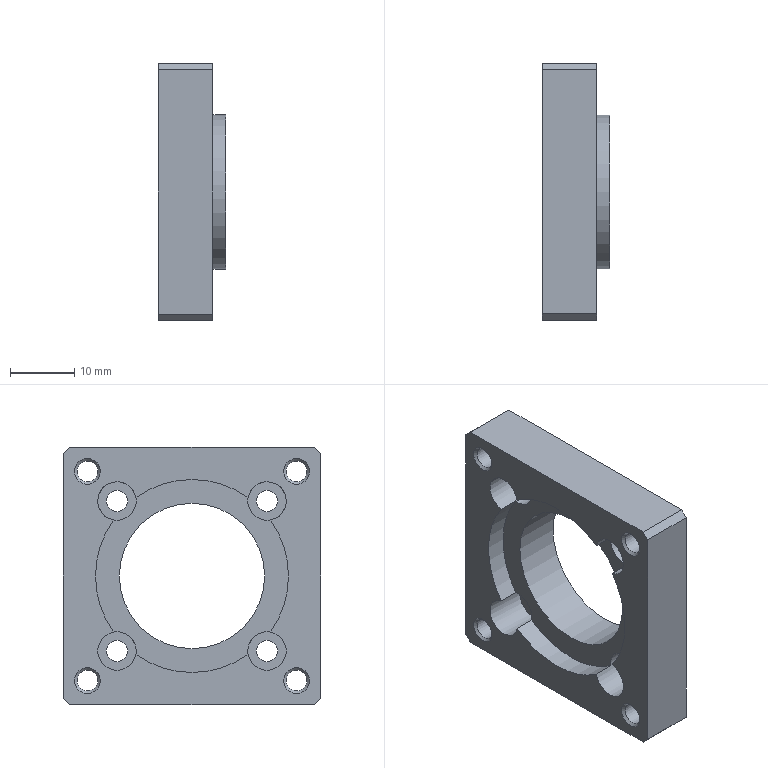Part | STEP file | C-KS50-F1_ma | 1 solid | 42 faces | box 10.5 x 40 x 40 mm | volume 8273 mm3 | cylinder 18 | plane 16 | cone 8 | commonest cylinder face diameters 3.242 x4 3.3 x4 6 x4 30 x4 22.6 x1 24 x1
STEP:
#1=CARTESIAN_POINT('',(-8.5,-12.208,8.716));
#2=VERTEX_POINT('',#1);
#3=CARTESIAN_POINT('',(-8.5,-12.208,-8.716));
#4=VERTEX_POINT('',#3);
#5=CARTESIAN_POINT('',(-8.5,0.,0.));
#6=DIRECTION('',(1.,0.,0.));
#7=DIRECTION('',(0.,0.,-1.));
#8=AXIS2_PLACEMENT_3D('',#5,#6,#7);
#9=CIRCLE('',#8,15.);
#10=EDGE_CURVE('',#2,#4,#9,.T.);
#11=ORIENTED_EDGE('',*,*,#10,.F.);
#12=CARTESIAN_POINT('',(-5.3,-12.208,8.716));
#13=VERTEX_POINT('',#12);
#14=CARTESIAN_POINT('',(-5.5,-12.208,8.716));
#15=DIRECTION('',(1.,0.,0.));
#16=VECTOR('',#15,1000.);
#17=LINE('',#14,#16);
#18=EDGE_CURVE('',#2,#13,#17,.T.);
#19=ORIENTED_EDGE('',*,*,#18,.T.);
#20=CARTESIAN_POINT('',(-5.3,-12.208,-8.716));
#21=VERTEX_POINT('',#20);
#22=CARTESIAN_POINT('',(-5.3,0.,0.));
#23=DIRECTION('',(1.,0.,0.));
#24=DIRECTION('',(0.,0.,-1.));
#25=AXIS2_PLACEMENT_3D('',#22,#23,#24);
#26=CIRCLE('',#25,15.);
#27=EDGE_CURVE('',#13,#21,#26,.T.);
#28=ORIENTED_EDGE('',*,*,#27,.T.);
#29=CARTESIAN_POINT('',(-5.5,-12.208,-8.716));
#30=DIRECTION('',(1.,0.,0.));
#31=VECTOR('',#30,1000.);
#32=LINE('',#29,#31);
#33=EDGE_CURVE('',#21,#4,#32,.F.);
#34=ORIENTED_EDGE('',*,*,#33,.T.);
#35=EDGE_LOOP('',(#11,#19,#28,#34));
#36=FACE_OUTER_BOUND('',#35,.T.);
#37=CARTESIAN_POINT('',(50.,0.,0.));
#38=DIRECTION('',(1.,0.,0.));
#39=DIRECTION('',(0.,0.,-1.));
#40=AXIS2_PLACEMENT_3D('',#37,#38,#39);
#41=CYLINDRICAL_SURFACE('',#40,15.);
#42=ADVANCED_FACE('',(#36),#41,.F.);
#43=CARTESIAN_POINT('',(-5.3,8.716,12.208));
#44=VERTEX_POINT('',#43);
#45=CARTESIAN_POINT('',(-5.3,-8.716,12.208));
#46=VERTEX_POINT('',#45);
#47=CARTESIAN_POINT('',(-5.3,0.,0.));
#48=DIRECTION('',(1.,0.,0.));
#49=DIRECTION('',(0.,0.,-1.));
#50=AXIS2_PLACEMENT_3D('',#47,#48,#49);
#51=CIRCLE('',#50,15.);
#52=EDGE_CURVE('',#44,#46,#51,.T.);
#53=ORIENTED_EDGE('',*,*,#52,.T.);
#54=CARTESIAN_POINT('',(-8.5,-8.716,12.208));
#55=VERTEX_POINT('',#54);
#56=CARTESIAN_POINT('',(-5.5,-8.716,12.208));
#57=DIRECTION('',(1.,0.,0.));
#58=VECTOR('',#57,1000.);
#59=LINE('',#56,#58);
#60=EDGE_CURVE('',#46,#55,#59,.F.);
#61=ORIENTED_EDGE('',*,*,#60,.T.);
#62=CARTESIAN_POINT('',(-8.5,8.716,12.208));
#63=VERTEX_POINT('',#62);
#64=CARTESIAN_POINT('',(-8.5,0.,0.));
#65=DIRECTION('',(1.,0.,0.));
#66=DIRECTION('',(0.,0.,-1.));
#67=AXIS2_PLACEMENT_3D('',#64,#65,#66);
#68=CIRCLE('',#67,15.);
#69=EDGE_CURVE('',#63,#55,#68,.T.);
#70=ORIENTED_EDGE('',*,*,#69,.F.);
#71=CARTESIAN_POINT('',(-5.5,8.716,12.208));
#72=DIRECTION('',(1.,0.,0.));
#73=VECTOR('',#72,1000.);
#74=LINE('',#71,#73);
#75=EDGE_CURVE('',#63,#44,#74,.T.);
#76=ORIENTED_EDGE('',*,*,#75,.T.);
#77=EDGE_LOOP('',(#53,#61,#70,#76));
#78=FACE_OUTER_BOUND('',#77,.T.);
#79=CARTESIAN_POINT('',(50.,0.,0.));
#80=DIRECTION('',(1.,0.,0.));
#81=DIRECTION('',(0.,0.,1.));
#82=AXIS2_PLACEMENT_3D('',#79,#80,#81);
#83=CYLINDRICAL_SURFACE('',#82,15.);
#84=ADVANCED_FACE('',(#78),#83,.F.);
#85=CARTESIAN_POINT('',(-8.5,-8.716,-12.208));
#86=VERTEX_POINT('',#85);
#87=CARTESIAN_POINT('',(-8.5,8.716,-12.208));
#88=VERTEX_POINT('',#87);
#89=CARTESIAN_POINT('',(-8.5,0.,0.));
#90=DIRECTION('',(1.,0.,0.));
#91=DIRECTION('',(0.,0.,-1.));
#92=AXIS2_PLACEMENT_3D('',#89,#90,#91);
#93=CIRCLE('',#92,15.);
#94=EDGE_CURVE('',#86,#88,#93,.T.);
#95=ORIENTED_EDGE('',*,*,#94,.F.);
#96=CARTESIAN_POINT('',(-5.3,-8.716,-12.208));
#97=VERTEX_POINT('',#96);
#98=CARTESIAN_POINT('',(-5.5,-8.716,-12.208));
#99=DIRECTION('',(1.,0.,0.));
#100=VECTOR('',#99,1000.);
#101=LINE('',#98,#100);
#102=EDGE_CURVE('',#86,#97,#101,.T.);
#103=ORIENTED_EDGE('',*,*,#102,.T.);
#104=CARTESIAN_POINT('',(-5.3,8.716,-12.208));
#105=VERTEX_POINT('',#104);
#106=CARTESIAN_POINT('',(-5.3,0.,0.));
#107=DIRECTION('',(1.,0.,0.));
#108=DIRECTION('',(0.,0.,-1.));
#109=AXIS2_PLACEMENT_3D('',#106,#107,#108);
#110=CIRCLE('',#109,15.);
#111=EDGE_CURVE('',#97,#105,#110,.T.);
#112=ORIENTED_EDGE('',*,*,#111,.T.);
#113=CARTESIAN_POINT('',(-5.5,8.716,-12.208));
#114=DIRECTION('',(1.,0.,0.));
#115=VECTOR('',#114,1000.);
#116=LINE('',#113,#115);
#117=EDGE_CURVE('',#105,#88,#116,.F.);
#118=ORIENTED_EDGE('',*,*,#117,.T.);
#119=EDGE_LOOP('',(#95,#103,#112,#118));
#120=FACE_OUTER_BOUND('',#119,.T.);
#121=CARTESIAN_POINT('',(50.,0.,0.));
#122=DIRECTION('',(1.,0.,0.));
#123=DIRECTION('',(0.,0.,-1.));
#124=AXIS2_PLACEMENT_3D('',#121,#122,#123);
#125=CYLINDRICAL_SURFACE('',#124,15.);
#126=ADVANCED_FACE('',(#120),#125,.F.);
#127=CARTESIAN_POINT('',(-5.3,12.208,-8.716));
#128=VERTEX_POINT('',#127);
#129=CARTESIAN_POINT('',(-5.3,12.208,8.716));
#130=VERTEX_POINT('',#129);
#131=CARTESIAN_POINT('',(-5.3,0.,0.));
#132=DIRECTION('',(1.,0.,0.));
#133=DIRECTION('',(0.,0.,-1.));
#134=AXIS2_PLACEMENT_3D('',#131,#132,#133);
#135=CIRCLE('',#134,15.);
#136=EDGE_CURVE('',#128,#130,#135,.T.);
#137=ORIENTED_EDGE('',*,*,#136,.T.);
#138=CARTESIAN_POINT('',(-8.5,12.208,8.716));
#139=VERTEX_POINT('',#138);
#140=CARTESIAN_POINT('',(-5.5,12.208,8.716));
#141=DIRECTION('',(1.,0.,0.));
#142=VECTOR('',#141,1000.);
#143=LINE('',#140,#142);
#144=EDGE_CURVE('',#130,#139,#143,.F.);
#145=ORIENTED_EDGE('',*,*,#144,.T.);
#146=CARTESIAN_POINT('',(-8.5,12.208,-8.716));
#147=VERTEX_POINT('',#146);
#148=CARTESIAN_POINT('',(-8.5,0.,0.));
#149=DIRECTION('',(1.,0.,0.));
#150=DIRECTION('',(0.,0.,-1.));
#151=AXIS2_PLACEMENT_3D('',#148,#149,#150);
#152=CIRCLE('',#151,15.);
#153=EDGE_CURVE('',#147,#139,#152,.T.);
#154=ORIENTED_EDGE('',*,*,#153,.F.);
#155=CARTESIAN_POINT('',(-5.5,12.208,-8.716));
#156=DIRECTION('',(1.,0.,0.));
#157=VECTOR('',#156,1000.);
#158=LINE('',#155,#157);
#159=EDGE_CURVE('',#147,#128,#158,.T.);
#160=ORIENTED_EDGE('',*,*,#159,.T.);
#161=EDGE_LOOP('',(#137,#145,#154,#160));
#162=FACE_OUTER_BOUND('',#161,.T.);
#163=CARTESIAN_POINT('',(50.,0.,0.));
#164=DIRECTION('',(1.,0.,0.));
#165=DIRECTION('',(0.,0.,-1.));
#166=AXIS2_PLACEMENT_3D('',#163,#164,#165);
#167=CYLINDRICAL_SURFACE('',#166,15.);
#168=ADVANCED_FACE('',(#162),#167,.F.);
#169=CARTESIAN_POINT('',(-8.5,20.,19.));
#170=VERTEX_POINT('',#169);
#171=CARTESIAN_POINT('',(-8.5,19.,20.));
#172=VERTEX_POINT('',#171);
#173=CARTESIAN_POINT('',(-8.5,44.5,-5.5));
#174=DIRECTION('',(0.,-0.7071,0.7071));
#175=VECTOR('',#174,1000.);
#176=LINE('',#173,#175);
#177=EDGE_CURVE('',#170,#172,#176,.T.);
#178=ORIENTED_EDGE('',*,*,#177,.F.);
#179=CARTESIAN_POINT('',(-8.5,20.,-19.));
#180=VERTEX_POINT('',#179);
#181=CARTESIAN_POINT('',(-8.5,20.,0.));
#182=DIRECTION('',(0.,0.,1.));
#183=VECTOR('',#182,1000.);
#184=LINE('',#181,#183);
#185=EDGE_CURVE('',#180,#170,#184,.T.);
#186=ORIENTED_EDGE('',*,*,#185,.F.);
#187=CARTESIAN_POINT('',(-8.5,19.,-20.));
#188=VERTEX_POINT('',#187);
#189=CARTESIAN_POINT('',(-8.5,44.5,5.5));
#190=DIRECTION('',(0.,0.7071,0.7071));
#191=VECTOR('',#190,1000.);
#192=LINE('',#189,#191);
#193=EDGE_CURVE('',#188,#180,#192,.T.);
#194=ORIENTED_EDGE('',*,*,#193,.F.);
#195=CARTESIAN_POINT('',(-8.5,-19.,-20.));
#196=VERTEX_POINT('',#195);
#197=CARTESIAN_POINT('',(-8.5,50.,-20.));
#198=DIRECTION('',(0.,1.,0.));
#199=VECTOR('',#198,1000.);
#200=LINE('',#197,#199);
#201=EDGE_CURVE('',#196,#188,#200,.T.);
#202=ORIENTED_EDGE('',*,*,#201,.F.);
#203=CARTESIAN_POINT('',(-8.5,-20.,-19.));
#204=VERTEX_POINT('',#203);
#205=CARTESIAN_POINT('',(-8.5,5.5,-44.5));
#206=DIRECTION('',(0.,0.7071,-0.7071));
#207=VECTOR('',#206,1000.);
#208=LINE('',#205,#207);
#209=EDGE_CURVE('',#204,#196,#208,.T.);
#210=ORIENTED_EDGE('',*,*,#209,.F.);
#211=CARTESIAN_POINT('',(-8.5,-20.,19.));
#212=VERTEX_POINT('',#211);
#213=CARTESIAN_POINT('',(-8.5,-20.,0.));
#214=DIRECTION('',(0.,0.,-1.));
#215=VECTOR('',#214,1000.);
#216=LINE('',#213,#215);
#217=EDGE_CURVE('',#212,#204,#216,.T.);
#218=ORIENTED_EDGE('',*,*,#217,.F.);
#219=CARTESIAN_POINT('',(-8.5,-19.,20.));
#220=VERTEX_POINT('',#219);
#221=CARTESIAN_POINT('',(-8.5,5.5,44.5));
#222=DIRECTION('',(0.,-0.7071,-0.7071));
#223=VECTOR('',#222,1000.);
#224=LINE('',#221,#223);
#225=EDGE_CURVE('',#220,#212,#224,.T.);
#226=ORIENTED_EDGE('',*,*,#225,.F.);
#227=CARTESIAN_POINT('',(-8.5,50.,20.));
#228=DIRECTION('',(0.,-1.,0.));
#229=VECTOR('',#228,1000.);
#230=LINE('',#227,#229);
#231=EDGE_CURVE('',#172,#220,#230,.T.);
#232=ORIENTED_EDGE('',*,*,#231,.F.);
#233=EDGE_LOOP('',(#178,#186,#194,#202,#210,#218,#226,#232));
#234=FACE_OUTER_BOUND('',#233,.T.);
#235=CARTESIAN_POINT('',(-8.5,11.667,-11.667));
#236=DIRECTION('',(-1.,0.,0.));
#237=DIRECTION('',(0.,0.,1.));
#238=AXIS2_PLACEMENT_3D('',#235,#236,#237);
#239=CIRCLE('',#238,3.);
#240=EDGE_CURVE('',#88,#147,#239,.F.);
#241=ORIENTED_EDGE('',*,*,#240,.T.);
#242=ORIENTED_EDGE('',*,*,#153,.T.);
#243=CARTESIAN_POINT('',(-8.5,11.667,14.667));
#244=VERTEX_POINT('',#243);
#245=CARTESIAN_POINT('',(-8.5,11.667,11.667));
#246=DIRECTION('',(-1.,0.,0.));
#247=DIRECTION('',(0.,0.,1.));
#248=AXIS2_PLACEMENT_3D('',#245,#246,#247);
#249=CIRCLE('',#248,3.);
#250=EDGE_CURVE('',#139,#244,#249,.F.);
#251=ORIENTED_EDGE('',*,*,#250,.T.);
#252=CARTESIAN_POINT('',(-8.5,11.667,11.667));
#253=DIRECTION('',(-1.,0.,0.));
#254=DIRECTION('',(0.,0.,1.));
#255=AXIS2_PLACEMENT_3D('',#252,#253,#254);
#256=CIRCLE('',#255,3.);
#257=EDGE_CURVE('',#244,#63,#256,.F.);
#258=ORIENTED_EDGE('',*,*,#257,.T.);
#259=ORIENTED_EDGE('',*,*,#69,.T.);
#260=CARTESIAN_POINT('',(-8.5,-11.667,14.667));
#261=VERTEX_POINT('',#260);
#262=CARTESIAN_POINT('',(-8.5,-11.667,11.667));
#263=DIRECTION('',(-1.,0.,0.));
#264=DIRECTION('',(0.,0.,1.));
#265=AXIS2_PLACEMENT_3D('',#262,#263,#264);
#266=CIRCLE('',#265,3.);
#267=EDGE_CURVE('',#55,#261,#266,.F.);
#268=ORIENTED_EDGE('',*,*,#267,.T.);
#269=CARTESIAN_POINT('',(-8.5,-11.667,11.667));
#270=DIRECTION('',(-1.,0.,0.));
#271=DIRECTION('',(0.,0.,1.));
#272=AXIS2_PLACEMENT_3D('',#269,#270,#271);
#273=CIRCLE('',#272,3.);
#274=EDGE_CURVE('',#261,#2,#273,.F.);
#275=ORIENTED_EDGE('',*,*,#274,.T.);
#276=ORIENTED_EDGE('',*,*,#10,.T.);
#277=CARTESIAN_POINT('',(-8.5,-11.667,-11.667));
#278=DIRECTION('',(-1.,0.,0.));
#279=DIRECTION('',(0.,0.,1.));
#280=AXIS2_PLACEMENT_3D('',#277,#278,#279);
#281=CIRCLE('',#280,3.);
#282=EDGE_CURVE('',#4,#86,#281,.F.);
#283=ORIENTED_EDGE('',*,*,#282,.T.);
#284=ORIENTED_EDGE('',*,*,#94,.T.);
#285=EDGE_LOOP('',(#241,#242,#251,#258,#259,#268,#275,#276,#283,#284));
#286=FACE_BOUND('',#285,.T.);
#287=CARTESIAN_POINT('',(-8.5,-16.263,14.263));
#288=VERTEX_POINT('',#287);
#289=CARTESIAN_POINT('',(-8.5,-16.263,16.263));
#290=DIRECTION('',(1.,0.,0.));
#291=DIRECTION('',(0.,0.,-1.));
#292=AXIS2_PLACEMENT_3D('',#289,#290,#291);
#293=CIRCLE('',#292,2.);
#294=EDGE_CURVE('',#288,#288,#293,.T.);
#295=ORIENTED_EDGE('',*,*,#294,.T.);
#296=EDGE_LOOP('',(#295));
#297=FACE_BOUND('',#296,.T.);
#298=CARTESIAN_POINT('',(-8.5,-16.263,-18.263));
#299=VERTEX_POINT('',#298);
#300=CARTESIAN_POINT('',(-8.5,-16.263,-16.263));
#301=DIRECTION('',(1.,0.,0.));
#302=DIRECTION('',(0.,0.,-1.));
#303=AXIS2_PLACEMENT_3D('',#300,#301,#302);
#304=CIRCLE('',#303,2.);
#305=EDGE_CURVE('',#299,#299,#304,.T.);
#306=ORIENTED_EDGE('',*,*,#305,.T.);
#307=EDGE_LOOP('',(#306));
#308=FACE_BOUND('',#307,.T.);
#309=CARTESIAN_POINT('',(-8.5,16.263,-18.263));
#310=VERTEX_POINT('',#309);
#311=CARTESIAN_POINT('',(-8.5,16.263,-16.263));
#312=DIRECTION('',(1.,0.,0.));
#313=DIRECTION('',(0.,0.,-1.));
#314=AXIS2_PLACEMENT_3D('',#311,#312,#313);
#315=CIRCLE('',#314,2.);
#316=EDGE_CURVE('',#310,#310,#315,.T.);
#317=ORIENTED_EDGE('',*,*,#316,.T.);
#318=EDGE_LOOP('',(#317));
#319=FACE_BOUND('',#318,.T.);
#320=CARTESIAN_POINT('',(-8.5,16.263,14.263));
#321=VERTEX_POINT('',#320);
#322=CARTESIAN_POINT('',(-8.5,16.263,16.263));
#323=DIRECTION('',(1.,0.,0.));
#324=DIRECTION('',(0.,0.,-1.));
#325=AXIS2_PLACEMENT_3D('',#322,#323,#324);
#326=CIRCLE('',#325,2.);
#327=EDGE_CURVE('',#321,#321,#326,.T.);
#328=ORIENTED_EDGE('',*,*,#327,.T.);
#329=EDGE_LOOP('',(#328));
#330=FACE_BOUND('',#329,.T.);
#331=CARTESIAN_POINT('',(-8.5,50.,0.));
#332=DIRECTION('',(-1.,0.,0.));
#333=DIRECTION('',(0.,0.,1.));
#334=AXIS2_PLACEMENT_3D('',#331,#332,#333);
#335=PLANE('',#334);
#336=ADVANCED_FACE('',(#234,#286,#297,#308,#319,#330),#335,.T.);
#337=ORIENTED_EDGE('',*,*,#27,.F.);
#338=CARTESIAN_POINT('',(-5.3,-11.667,11.667));
#339=DIRECTION('',(-1.,0.,0.));
#340=DIRECTION('',(0.,0.,1.));
#341=AXIS2_PLACEMENT_3D('',#338,#339,#340);
#342=CIRCLE('',#341,3.);
#343=EDGE_CURVE('',#13,#46,#342,.F.);
#344=ORIENTED_EDGE('',*,*,#343,.T.);
#345=ORIENTED_EDGE('',*,*,#52,.F.);
#346=CARTESIAN_POINT('',(-5.3,11.667,11.667));
#347=DIRECTION('',(-1.,0.,0.));
#348=DIRECTION('',(0.,0.,1.));
#349=AXIS2_PLACEMENT_3D('',#346,#347,#348);
#350=CIRCLE('',#349,3.);
#351=EDGE_CURVE('',#44,#130,#350,.F.);
#352=ORIENTED_EDGE('',*,*,#351,.T.);
#353=ORIENTED_EDGE('',*,*,#136,.F.);
#354=CARTESIAN_POINT('',(-5.3,11.667,-8.667));
#355=VERTEX_POINT('',#354);
#356=CARTESIAN_POINT('',(-5.3,11.667,-11.667));
#357=DIRECTION('',(-1.,0.,0.));
#358=DIRECTION('',(0.,0.,1.));
#359=AXIS2_PLACEMENT_3D('',#356,#357,#358);
#360=CIRCLE('',#359,3.);
#361=EDGE_CURVE('',#128,#355,#360,.F.);
#362=ORIENTED_EDGE('',*,*,#361,.T.);
#363=CARTESIAN_POINT('',(-5.3,11.667,-11.667));
#364=DIRECTION('',(-1.,0.,0.));
#365=DIRECTION('',(0.,0.,1.));
#366=AXIS2_PLACEMENT_3D('',#363,#364,#365);
#367=CIRCLE('',#366,3.);
#368=EDGE_CURVE('',#355,#105,#367,.F.);
#369=ORIENTED_EDGE('',*,*,#368,.T.);
#370=ORIENTED_EDGE('',*,*,#111,.F.);
#371=CARTESIAN_POINT('',(-5.3,-11.667,-8.667));
#372=VERTEX_POINT('',#371);
#373=CARTESIAN_POINT('',(-5.3,-11.667,-11.667));
#374=DIRECTION('',(-1.,0.,0.));
#375=DIRECTION('',(0.,0.,1.));
#376=AXIS2_PLACEMENT_3D('',#373,#374,#375);
#377=CIRCLE('',#376,3.);
#378=EDGE_CURVE('',#97,#372,#377,.F.);
#379=ORIENTED_EDGE('',*,*,#378,.T.);
#380=CARTESIAN_POINT('',(-5.3,-11.667,-11.667));
#381=DIRECTION('',(-1.,0.,0.));
#382=DIRECTION('',(0.,0.,1.));
#383=AXIS2_PLACEMENT_3D('',#380,#381,#382);
#384=CIRCLE('',#383,3.);
#385=EDGE_CURVE('',#372,#21,#384,.F.);
#386=ORIENTED_EDGE('',*,*,#385,.T.);
#387=EDGE_LOOP('',(#337,#344,#345,#352,#353,#362,#369,#370,#379,#386));
#388=FACE_OUTER_BOUND('',#387,.T.);
#389=CARTESIAN_POINT('',(-5.3,0.,-11.3));
#390=VERTEX_POINT('',#389);
#391=CARTESIAN_POINT('',(-5.3,0.,11.3));
#392=VERTEX_POINT('',#391);
#393=CARTESIAN_POINT('',(-5.3,0.,0.));
#394=DIRECTION('',(1.,0.,0.));
#395=DIRECTION('',(0.,0.,-1.));
#396=AXIS2_PLACEMENT_3D('',#393,#394,#395);
#397=CIRCLE('',#396,11.3);
#398=EDGE_CURVE('',#390,#392,#397,.T.);
#399=ORIENTED_EDGE('',*,*,#398,.T.);
#400=CARTESIAN_POINT('',(-5.3,0.,0.));
#401=DIRECTION('',(1.,0.,0.));
#402=DIRECTION('',(0.,0.,-1.));
#403=AXIS2_PLACEMENT_3D('',#400,#401,#402);
#404=CIRCLE('',#403,11.3);
#405=EDGE_CURVE('',#392,#390,#404,.T.);
#406=ORIENTED_EDGE('',*,*,#405,.T.);
#407=EDGE_LOOP('',(#399,#406));
#408=FACE_BOUND('',#407,.T.);
#409=CARTESIAN_POINT('',(-5.3,15.,0.));
#410=DIRECTION('',(-1.,0.,0.));
#411=DIRECTION('',(0.,0.,1.));
#412=AXIS2_PLACEMENT_3D('',#409,#410,#411);
#413=PLANE('',#412);
#414=ADVANCED_FACE('',(#388,#408),#413,.T.);
#415=ORIENTED_EDGE('',*,*,#398,.F.);
#416=ORIENTED_EDGE('',*,*,#405,.F.);
#417=CARTESIAN_POINT('',(2.,0.,11.3));
#418=VERTEX_POINT('',#417);
#419=CARTESIAN_POINT('',(50.,0.,11.3));
#420=DIRECTION('',(1.,0.,0.));
#421=VECTOR('',#420,11.3);
#422=LINE('',#419,#421);
#423=EDGE_CURVE('',#392,#418,#422,.T.);
#424=ORIENTED_EDGE('',*,*,#423,.T.);
#425=CARTESIAN_POINT('',(2.,0.,-11.3));
#426=VERTEX_POINT('',#425);
#427=CARTESIAN_POINT('',(2.,0.,0.));
#428=DIRECTION('',(1.,0.,0.));
#429=DIRECTION('',(0.,0.,-1.));
#430=AXIS2_PLACEMENT_3D('',#427,#428,#429);
#431=CIRCLE('',#430,11.3);
#432=EDGE_CURVE('',#418,#426,#431,.T.);
#433=ORIENTED_EDGE('',*,*,#432,.T.);
#434=CARTESIAN_POINT('',(2.,0.,0.));
#435=DIRECTION('',(1.,0.,0.));
#436=DIRECTION('',(0.,0.,-1.));
#437=AXIS2_PLACEMENT_3D('',#434,#435,#436);
#438=CIRCLE('',#437,11.3);
#439=EDGE_CURVE('',#426,#418,#438,.T.);
#440=ORIENTED_EDGE('',*,*,#439,.T.);
#441=ORIENTED_EDGE('',*,*,#423,.F.);
#442=EDGE_LOOP('',(#415,#416,#424,#433,#440,#441));
#443=FACE_OUTER_BOUND('',#442,.T.);
#444=CARTESIAN_POINT('',(50.,0.,0.));
#445=DIRECTION('',(1.,0.,0.));
#446=DIRECTION('',(0.,0.,-1.));
#447=AXIS2_PLACEMENT_3D('',#444,#445,#446);
#448=CYLINDRICAL_SURFACE('',#447,11.3);
#449=ADVANCED_FACE('',(#443),#448,.F.);
#450=CARTESIAN_POINT('',(2.,0.,-12.));
#451=VERTEX_POINT('',#450);
#452=CARTESIAN_POINT('',(2.,0.,12.));
#453=VERTEX_POINT('',#452);
#454=CARTESIAN_POINT('',(2.,0.,0.));
#455=DIRECTION('',(1.,0.,0.));
#456=DIRECTION('',(0.,0.,-1.));
#457=AXIS2_PLACEMENT_3D('',#454,#455,#456);
#458=CIRCLE('',#457,12.);
#459=EDGE_CURVE('',#451,#453,#458,.T.);
#460=ORIENTED_EDGE('',*,*,#459,.T.);
#461=CARTESIAN_POINT('',(2.,0.,0.));
#462=DIRECTION('',(1.,0.,0.));
#463=DIRECTION('',(0.,0.,-1.));
#464=AXIS2_PLACEMENT_3D('',#461,#462,#463);
#465=CIRCLE('',#464,12.);
#466=EDGE_CURVE('',#453,#451,#465,.T.);
#467=ORIENTED_EDGE('',*,*,#466,.T.);
#468=EDGE_LOOP('',(#460,#467));
#469=FACE_OUTER_BOUND('',#468,.T.);
#470=ORIENTED_EDGE('',*,*,#439,.F.);
#471=ORIENTED_EDGE('',*,*,#432,.F.);
#472=EDGE_LOOP('',(#470,#471));
#473=FACE_BOUND('',#472,.T.);
#474=CARTESIAN_POINT('',(2.,11.3,0.));
#475=DIRECTION('',(1.,0.,0.));
#476=DIRECTION('',(0.,0.,-1.));
#477=AXIS2_PLACEMENT_3D('',#474,#475,#476);
#478=PLANE('',#477);
#479=ADVANCED_FACE('',(#469,#473),#478,.T.);
#480=ORIENTED_EDGE('',*,*,#459,.F.);
#481=ORIENTED_EDGE('',*,*,#466,.F.);
#482=CARTESIAN_POINT('',(0.,0.,12.));
#483=VERTEX_POINT('',#482);
#484=CARTESIAN_POINT('',(50.,0.,12.));
#485=DIRECTION('',(-1.,0.,0.));
#486=VECTOR('',#485,12.);
#487=LINE('',#484,#486);
#488=EDGE_CURVE('',#453,#483,#487,.T.);
#489=ORIENTED_EDGE('',*,*,#488,.T.);
#490=CARTESIAN_POINT('',(0.,0.,-12.));
#491=VERTEX_POINT('',#490);
#492=CARTESIAN_POINT('',(0.,0.,0.));
#493=DIRECTION('',(1.,0.,0.));
#494=DIRECTION('',(0.,0.,-1.));
#495=AXIS2_PLACEMENT_3D('',#492,#493,#494);
#496=CIRCLE('',#495,12.);
#497=EDGE_CURVE('',#483,#491,#496,.T.);
#498=ORIENTED_EDGE('',*,*,#497,.T.);
#499=CARTESIAN_POINT('',(0.,0.,0.));
#500=DIRECTION('',(1.,0.,0.));
#501=DIRECTION('',(0.,0.,-1.));
#502=AXIS2_PLACEMENT_3D('',#499,#500,#501);
#503=CIRCLE('',#502,12.);
#504=EDGE_CURVE('',#491,#483,#503,.T.);
#505=ORIENTED_EDGE('',*,*,#504,.T.);
#506=ORIENTED_EDGE('',*,*,#488,.F.);
#507=EDGE_LOOP('',(#480,#481,#489,#498,#505,#506));
#508=FACE_OUTER_BOUND('',#507,.T.);
#509=CARTESIAN_POINT('',(50.,0.,0.));
#510=DIRECTION('',(1.,0.,0.));
#511=DIRECTION('',(0.,0.,-1.));
#512=AXIS2_PLACEMENT_3D('',#509,#510,#511);
#513=CYLINDRICAL_SURFACE('',#512,12.);
#514=ADVANCED_FACE('',(#508),#513,.T.);
#515=CARTESIAN_POINT('',(0.,20.,19.));
#516=VERTEX_POINT('',#515);
#517=CARTESIAN_POINT('',(0.,20.,-19.));
#518=VERTEX_POINT('',#517);
#519=CARTESIAN_POINT('',(0.,20.,0.));
#520=DIRECTION('',(0.,0.,-1.));
#521=VECTOR('',#520,1000.);
#522=LINE('',#519,#521);
#523=EDGE_CURVE('',#516,#518,#522,.T.);
#524=ORIENTED_EDGE('',*,*,#523,.F.);
#525=CARTESIAN_POINT('',(0.,19.,20.));
#526=VERTEX_POINT('',#525);
#527=CARTESIAN_POINT('',(0.,25.5,13.5));
#528=DIRECTION('',(0.,0.7071,-0.7071));
#529=VECTOR('',#528,1000.);
#530=LINE('',#527,#529);
#531=EDGE_CURVE('',#526,#516,#530,.T.);
#532=ORIENTED_EDGE('',*,*,#531,.F.);
#533=CARTESIAN_POINT('',(0.,-19.,20.));
#534=VERTEX_POINT('',#533);
#535=CARTESIAN_POINT('',(0.,12.,20.));
#536=DIRECTION('',(0.,1.,0.));
#537=VECTOR('',#536,1000.);
#538=LINE('',#535,#537);
#539=EDGE_CURVE('',#534,#526,#538,.T.);
#540=ORIENTED_EDGE('',*,*,#539,.F.);
#541=CARTESIAN_POINT('',(0.,-20.,19.));
#542=VERTEX_POINT('',#541);
#543=CARTESIAN_POINT('',(0.,-13.5,25.5));
#544=DIRECTION('',(0.,0.7071,0.7071));
#545=VECTOR('',#544,1000.);
#546=LINE('',#543,#545);
#547=EDGE_CURVE('',#542,#534,#546,.T.);
#548=ORIENTED_EDGE('',*,*,#547,.F.);
#549=CARTESIAN_POINT('',(0.,-20.,-19.));
#550=VERTEX_POINT('',#549);
#551=CARTESIAN_POINT('',(0.,-20.,0.));
#552=DIRECTION('',(0.,0.,1.));
#553=VECTOR('',#552,1000.);
#554=LINE('',#551,#553);
#555=EDGE_CURVE('',#550,#542,#554,.T.);
#556=ORIENTED_EDGE('',*,*,#555,.F.);
#557=CARTESIAN_POINT('',(0.,-19.,-20.));
#558=VERTEX_POINT('',#557);
#559=CARTESIAN_POINT('',(0.,-13.5,-25.5));
#560=DIRECTION('',(0.,-0.7071,0.7071));
#561=VECTOR('',#560,1000.);
#562=LINE('',#559,#561);
#563=EDGE_CURVE('',#558,#550,#562,.T.);
#564=ORIENTED_EDGE('',*,*,#563,.F.);
#565=CARTESIAN_POINT('',(0.,19.,-20.));
#566=VERTEX_POINT('',#565);
#567=CARTESIAN_POINT('',(0.,12.,-20.));
#568=DIRECTION('',(0.,-1.,0.));
#569=VECTOR('',#568,1000.);
#570=LINE('',#567,#569);
#571=EDGE_CURVE('',#566,#558,#570,.T.);
#572=ORIENTED_EDGE('',*,*,#571,.F.);
#573=CARTESIAN_POINT('',(0.,25.5,-13.5));
#574=DIRECTION('',(0.,-0.7071,-0.7071));
#575=VECTOR('',#574,1000.);
#576=LINE('',#573,#575);
#577=EDGE_CURVE('',#518,#566,#576,.T.);
#578=ORIENTED_EDGE('',*,*,#577,.F.);
#579=EDGE_LOOP('',(#524,#532,#540,#548,#556,#564,#572,#578));
#580=FACE_OUTER_BOUND('',#579,.T.);
#581=CARTESIAN_POINT('',(0.,-16.263,14.263));
#582=VERTEX_POINT('',#581);
#583=CARTESIAN_POINT('',(0.,-16.263,18.263));
#584=VERTEX_POINT('',#583);
#585=CARTESIAN_POINT('',(0.,-16.263,16.263));
#586=DIRECTION('',(1.,0.,0.));
#587=DIRECTION('',(0.,0.,-1.));
#588=AXIS2_PLACEMENT_3D('',#585,#586,#587);
#589=CIRCLE('',#588,2.);
#590=EDGE_CURVE('',#582,#584,#589,.T.);
#591=ORIENTED_EDGE('',*,*,#590,.F.);
#592=CARTESIAN_POINT('',(0.,-16.263,16.263));
#593=DIRECTION('',(1.,0.,0.));
#594=DIRECTION('',(0.,0.,-1.));
#595=AXIS2_PLACEMENT_3D('',#592,#593,#594);
#596=CIRCLE('',#595,2.);
#597=EDGE_CURVE('',#584,#582,#596,.T.);
#598=ORIENTED_EDGE('',*,*,#597,.F.);
#599=EDGE_LOOP('',(#591,#598));
#600=FACE_BOUND('',#599,.T.);
#601=CARTESIAN_POINT('',(0.,-16.263,-18.263));
#602=VERTEX_POINT('',#601);
#603=CARTESIAN_POINT('',(0.,-16.263,-14.263));
#604=VERTEX_POINT('',#603);
#605=CARTESIAN_POINT('',(0.,-16.263,-16.263));
#606=DIRECTION('',(1.,0.,0.));
#607=DIRECTION('',(0.,0.,-1.));
#608=AXIS2_PLACEMENT_3D('',#605,#606,#607);
#609=CIRCLE('',#608,2.);
#610=EDGE_CURVE('',#602,#604,#609,.T.);
#611=ORIENTED_EDGE('',*,*,#610,.F.);
#612=CARTESIAN_POINT('',(0.,-16.263,-16.263));
#613=DIRECTION('',(1.,0.,0.));
#614=DIRECTION('',(0.,0.,-1.));
#615=AXIS2_PLACEMENT_3D('',#612,#613,#614);
#616=CIRCLE('',#615,2.);
#617=EDGE_CURVE('',#604,#602,#616,.T.);
#618=ORIENTED_EDGE('',*,*,#617,.F.);
#619=EDGE_LOOP('',(#611,#618));
#620=FACE_BOUND('',#619,.T.);
#621=CARTESIAN_POINT('',(0.,16.263,-18.263));
#622=VERTEX_POINT('',#621);
#623=CARTESIAN_POINT('',(0.,16.263,-14.263));
#624=VERTEX_POINT('',#623);
#625=CARTESIAN_POINT('',(0.,16.263,-16.263));
#626=DIRECTION('',(1.,0.,0.));
#627=DIRECTION('',(0.,0.,-1.));
#628=AXIS2_PLACEMENT_3D('',#625,#626,#627);
#629=CIRCLE('',#628,2.);
#630=EDGE_CURVE('',#622,#624,#629,.T.);
#631=ORIENTED_EDGE('',*,*,#630,.F.);
#632=CARTESIAN_POINT('',(0.,16.263,-16.263));
#633=DIRECTION('',(1.,0.,0.));
#634=DIRECTION('',(0.,0.,-1.));
#635=AXIS2_PLACEMENT_3D('',#632,#633,#634);
#636=CIRCLE('',#635,2.);
#637=EDGE_CURVE('',#624,#622,#636,.T.);
#638=ORIENTED_EDGE('',*,*,#637,.F.);
#639=EDGE_LOOP('',(#631,#638));
#640=FACE_BOUND('',#639,.T.);
#641=CARTESIAN_POINT('',(0.,16.263,14.263));
#642=VERTEX_POINT('',#641);
#643=CARTESIAN_POINT('',(0.,16.263,18.263));
#644=VERTEX_POINT('',#643);
#645=CARTESIAN_POINT('',(0.,16.263,16.263));
#646=DIRECTION('',(1.,0.,0.));
#647=DIRECTION('',(0.,0.,-1.));
#648=AXIS2_PLACEMENT_3D('',#645,#646,#647);
#649=CIRCLE('',#648,2.);
#650=EDGE_CURVE('',#642,#644,#649,.T.);
#651=ORIENTED_EDGE('',*,*,#650,.F.);
#652=CARTESIAN_POINT('',(0.,16.263,16.263));
#653=DIRECTION('',(1.,0.,0.));
#654=DIRECTION('',(0.,0.,-1.));
#655=AXIS2_PLACEMENT_3D('',#652,#653,#654);
#656=CIRCLE('',#655,2.);
#657=EDGE_CURVE('',#644,#642,#656,.T.);
#658=ORIENTED_EDGE('',*,*,#657,.F.);
#659=EDGE_LOOP('',(#651,#658));
#660=FACE_BOUND('',#659,.T.);
#661=CARTESIAN_POINT('',(0.,-11.667,10.017));
#662=VERTEX_POINT('',#661);
#663=CARTESIAN_POINT('',(0.,-11.667,13.317));
#664=VERTEX_POINT('',#663);
#665=CARTESIAN_POINT('',(0.,-11.667,11.667));
#666=DIRECTION('',(1.,0.,0.));
#667=DIRECTION('',(0.,0.,-1.));
#668=AXIS2_PLACEMENT_3D('',#665,#666,#667);
#669=CIRCLE('',#668,1.65);
#670=EDGE_CURVE('',#662,#664,#669,.T.);
#671=ORIENTED_EDGE('',*,*,#670,.F.);
#672=CARTESIAN_POINT('',(0.,-11.667,11.667));
#673=DIRECTION('',(1.,0.,0.));
#674=DIRECTION('',(0.,0.,-1.));
#675=AXIS2_PLACEMENT_3D('',#672,#673,#674);
#676=CIRCLE('',#675,1.65);
#677=EDGE_CURVE('',#664,#662,#676,.T.);
#678=ORIENTED_EDGE('',*,*,#677,.F.);
#679=EDGE_LOOP('',(#671,#678));
#680=FACE_BOUND('',#679,.T.);
#681=CARTESIAN_POINT('',(0.,-11.667,-13.317));
#682=VERTEX_POINT('',#681);
#683=CARTESIAN_POINT('',(0.,-11.667,-10.017));
#684=VERTEX_POINT('',#683);
#685=CARTESIAN_POINT('',(0.,-11.667,-11.667));
#686=DIRECTION('',(1.,0.,0.));
#687=DIRECTION('',(0.,0.,-1.));
#688=AXIS2_PLACEMENT_3D('',#685,#686,#687);
#689=CIRCLE('',#688,1.65);
#690=EDGE_CURVE('',#682,#684,#689,.T.);
#691=ORIENTED_EDGE('',*,*,#690,.F.);
#692=CARTESIAN_POINT('',(0.,-11.667,-11.667));
#693=DIRECTION('',(1.,0.,0.));
#694=DIRECTION('',(0.,0.,-1.));
#695=AXIS2_PLACEMENT_3D('',#692,#693,#694);
#696=CIRCLE('',#695,1.65);
#697=EDGE_CURVE('',#684,#682,#696,.T.);
#698=ORIENTED_EDGE('',*,*,#697,.F.);
#699=EDGE_LOOP('',(#691,#698));
#700=FACE_BOUND('',#699,.T.);
#701=CARTESIAN_POINT('',(0.,11.667,-13.317));
#702=VERTEX_POINT('',#701);
#703=CARTESIAN_POINT('',(0.,11.667,-10.017));
#704=VERTEX_POINT('',#703);
#705=CARTESIAN_POINT('',(0.,11.667,-11.667));
#706=DIRECTION('',(1.,0.,0.));
#707=DIRECTION('',(0.,0.,-1.));
#708=AXIS2_PLACEMENT_3D('',#705,#706,#707);
#709=CIRCLE('',#708,1.65);
#710=EDGE_CURVE('',#702,#704,#709,.T.);
#711=ORIENTED_EDGE('',*,*,#710,.F.);
#712=CARTESIAN_POINT('',(0.,11.667,-11.667));
#713=DIRECTION('',(1.,0.,0.));
#714=DIRECTION('',(0.,0.,-1.));
#715=AXIS2_PLACEMENT_3D('',#712,#713,#714);
#716=CIRCLE('',#715,1.65);
#717=EDGE_CURVE('',#704,#702,#716,.T.);
#718=ORIENTED_EDGE('',*,*,#717,.F.);
#719=EDGE_LOOP('',(#711,#718));
#720=FACE_BOUND('',#719,.T.);
#721=CARTESIAN_POINT('',(0.,11.667,10.017));
#722=VERTEX_POINT('',#721);
#723=CARTESIAN_POINT('',(0.,11.667,13.317));
#724=VERTEX_POINT('',#723);
#725=CARTESIAN_POINT('',(0.,11.667,11.667));
#726=DIRECTION('',(1.,0.,0.));
#727=DIRECTION('',(0.,0.,-1.));
#728=AXIS2_PLACEMENT_3D('',#725,#726,#727);
#729=CIRCLE('',#728,1.65);
#730=EDGE_CURVE('',#722,#724,#729,.T.);
#731=ORIENTED_EDGE('',*,*,#730,.F.);
#732=CARTESIAN_POINT('',(0.,11.667,11.667));
#733=DIRECTION('',(1.,0.,0.));
#734=DIRECTION('',(0.,0.,-1.));
#735=AXIS2_PLACEMENT_3D('',#732,#733,#734);
#736=CIRCLE('',#735,1.65);
#737=EDGE_CURVE('',#724,#722,#736,.T.);
#738=ORIENTED_EDGE('',*,*,#737,.F.);
#739=EDGE_LOOP('',(#731,#738));
#740=FACE_BOUND('',#739,.T.);
#741=ORIENTED_EDGE('',*,*,#504,.F.);
#742=ORIENTED_EDGE('',*,*,#497,.F.);
#743=EDGE_LOOP('',(#741,#742));
#744=FACE_BOUND('',#743,.T.);
#745=CARTESIAN_POINT('',(0.,12.,0.));
#746=DIRECTION('',(1.,0.,0.));
#747=DIRECTION('',(0.,0.,-1.));
#748=AXIS2_PLACEMENT_3D('',#745,#746,#747);
#749=PLANE('',#748);
#750=ADVANCED_FACE('',(#580,#600,#620,#640,#660,#680,#700,#720,#740,#744),#749,.T.);
#751=ORIENTED_EDGE('',*,*,#177,.T.);
#752=CARTESIAN_POINT('',(10.,19.,20.));
#753=DIRECTION('',(-1.,0.,0.));
#754=VECTOR('',#753,1000.);
#755=LINE('',#752,#754);
#756=EDGE_CURVE('',#526,#172,#755,.T.);
#757=ORIENTED_EDGE('',*,*,#756,.F.);
#758=ORIENTED_EDGE('',*,*,#531,.T.);
#759=CARTESIAN_POINT('',(10.,20.,19.));
#760=DIRECTION('',(-1.,0.,0.));
#761=VECTOR('',#760,1000.);
#762=LINE('',#759,#761);
#763=EDGE_CURVE('',#516,#170,#762,.T.);
#764=ORIENTED_EDGE('',*,*,#763,.T.);
#765=EDGE_LOOP('',(#751,#757,#758,#764));
#766=FACE_OUTER_BOUND('',#765,.T.);
#767=CARTESIAN_POINT('',(10.,20.,19.));
#768=DIRECTION('',(0.,-0.7071,-0.7071));
#769=DIRECTION('',(0.,0.7071,-0.7071));
#770=AXIS2_PLACEMENT_3D('',#767,#768,#769);
#771=PLANE('',#770);
#772=ADVANCED_FACE('',(#766),#771,.F.);
#773=ORIENTED_EDGE('',*,*,#185,.T.);
#774=ORIENTED_EDGE('',*,*,#763,.F.);
#775=ORIENTED_EDGE('',*,*,#523,.T.);
#776=CARTESIAN_POINT('',(10.,20.,-19.));
#777=DIRECTION('',(-1.,0.,0.));
#778=VECTOR('',#777,1000.);
#779=LINE('',#776,#778);
#780=EDGE_CURVE('',#518,#180,#779,.T.);
#781=ORIENTED_EDGE('',*,*,#780,.T.);
#782=EDGE_LOOP('',(#773,#774,#775,#781));
#783=FACE_OUTER_BOUND('',#782,.T.);
#784=CARTESIAN_POINT('',(10.,20.,-19.));
#785=DIRECTION('',(0.,-1.,0.));
#786=DIRECTION('',(0.,0.,-1.));
#787=AXIS2_PLACEMENT_3D('',#784,#785,#786);
#788=PLANE('',#787);
#789=ADVANCED_FACE('',(#783),#788,.F.);
#790=ORIENTED_EDGE('',*,*,#193,.T.);
#791=ORIENTED_EDGE('',*,*,#780,.F.);
#792=ORIENTED_EDGE('',*,*,#577,.T.);
#793=CARTESIAN_POINT('',(10.,19.,-20.));
#794=DIRECTION('',(-1.,0.,0.));
#795=VECTOR('',#794,1000.);
#796=LINE('',#793,#795);
#797=EDGE_CURVE('',#566,#188,#796,.T.);
#798=ORIENTED_EDGE('',*,*,#797,.T.);
#799=EDGE_LOOP('',(#790,#791,#792,#798));
#800=FACE_OUTER_BOUND('',#799,.T.);
#801=CARTESIAN_POINT('',(10.,19.,-20.));
#802=DIRECTION('',(0.,-0.7071,0.7071));
#803=DIRECTION('',(0.,-0.7071,-0.7071));
#804=AXIS2_PLACEMENT_3D('',#801,#802,#803);
#805=PLANE('',#804);
#806=ADVANCED_FACE('',(#800),#805,.F.);
#807=ORIENTED_EDGE('',*,*,#201,.T.);
#808=ORIENTED_EDGE('',*,*,#797,.F.);
#809=ORIENTED_EDGE('',*,*,#571,.T.);
#810=CARTESIAN_POINT('',(10.,-19.,-20.));
#811=DIRECTION('',(-1.,0.,0.));
#812=VECTOR('',#811,1000.);
#813=LINE('',#810,#812);
#814=EDGE_CURVE('',#558,#196,#813,.T.);
#815=ORIENTED_EDGE('',*,*,#814,.T.);
#816=EDGE_LOOP('',(#807,#808,#809,#815));
#817=FACE_OUTER_BOUND('',#816,.T.);
#818=CARTESIAN_POINT('',(10.,-19.,-20.));
#819=DIRECTION('',(0.,0.,1.));
#820=DIRECTION('',(1.,0.,0.));
#821=AXIS2_PLACEMENT_3D('',#818,#819,#820);
#822=PLANE('',#821);
#823=ADVANCED_FACE('',(#817),#822,.F.);
#824=ORIENTED_EDGE('',*,*,#209,.T.);
#825=ORIENTED_EDGE('',*,*,#814,.F.);
#826=ORIENTED_EDGE('',*,*,#563,.T.);
#827=CARTESIAN_POINT('',(10.,-20.,-19.));
#828=DIRECTION('',(-1.,0.,0.));
#829=VECTOR('',#828,1000.);
#830=LINE('',#827,#829);
#831=EDGE_CURVE('',#550,#204,#830,.T.);
#832=ORIENTED_EDGE('',*,*,#831,.T.);
#833=EDGE_LOOP('',(#824,#825,#826,#832));
#834=FACE_OUTER_BOUND('',#833,.T.);
#835=CARTESIAN_POINT('',(10.,-20.,-19.));
#836=DIRECTION('',(0.,0.7071,0.7071));
#837=DIRECTION('',(0.,-0.7071,0.7071));
#838=AXIS2_PLACEMENT_3D('',#835,#836,#837);
#839=PLANE('',#838);
#840=ADVANCED_FACE('',(#834),#839,.F.);
#841=ORIENTED_EDGE('',*,*,#217,.T.);
#842=ORIENTED_EDGE('',*,*,#831,.F.);
#843=ORIENTED_EDGE('',*,*,#555,.T.);
#844=CARTESIAN_POINT('',(10.,-20.,19.));
#845=DIRECTION('',(-1.,0.,0.));
#846=VECTOR('',#845,1000.);
#847=LINE('',#844,#846);
#848=EDGE_CURVE('',#542,#212,#847,.T.);
#849=ORIENTED_EDGE('',*,*,#848,.T.);
#850=EDGE_LOOP('',(#841,#842,#843,#849));
#851=FACE_OUTER_BOUND('',#850,.T.);
#852=CARTESIAN_POINT('',(10.,-20.,19.));
#853=DIRECTION('',(0.,1.,0.));
#854=DIRECTION('',(0.,0.,1.));
#855=AXIS2_PLACEMENT_3D('',#852,#853,#854);
#856=PLANE('',#855);
#857=ADVANCED_FACE('',(#851),#856,.F.);
#858=ORIENTED_EDGE('',*,*,#225,.T.);
#859=ORIENTED_EDGE('',*,*,#848,.F.);
#860=ORIENTED_EDGE('',*,*,#547,.T.);
#861=CARTESIAN_POINT('',(10.,-19.,20.));
#862=DIRECTION('',(-1.,0.,0.));
#863=VECTOR('',#862,1000.);
#864=LINE('',#861,#863);
#865=EDGE_CURVE('',#534,#220,#864,.T.);
#866=ORIENTED_EDGE('',*,*,#865,.T.);
#867=EDGE_LOOP('',(#858,#859,#860,#866));
#868=FACE_OUTER_BOUND('',#867,.T.);
#869=CARTESIAN_POINT('',(10.,-19.,20.));
#870=DIRECTION('',(0.,0.7071,-0.7071));
#871=DIRECTION('',(0.,0.7071,0.7071));
#872=AXIS2_PLACEMENT_3D('',#869,#870,#871);
#873=PLANE('',#872);
#874=ADVANCED_FACE('',(#868),#873,.F.);
#875=ORIENTED_EDGE('',*,*,#231,.T.);
#876=ORIENTED_EDGE('',*,*,#865,.F.);
#877=ORIENTED_EDGE('',*,*,#539,.T.);
#878=ORIENTED_EDGE('',*,*,#756,.T.);
#879=EDGE_LOOP('',(#875,#876,#877,#878));
#880=FACE_OUTER_BOUND('',#879,.T.);
#881=CARTESIAN_POINT('',(10.,19.,20.));
#882=DIRECTION('',(0.,0.,-1.));
#883=DIRECTION('',(-1.,0.,0.));
#884=AXIS2_PLACEMENT_3D('',#881,#882,#883);
#885=PLANE('',#884);
#886=ADVANCED_FACE('',(#880),#885,.F.);
#887=ORIENTED_EDGE('',*,*,#250,.F.);
#888=ORIENTED_EDGE('',*,*,#144,.F.);
#889=ORIENTED_EDGE('',*,*,#351,.F.);
#890=ORIENTED_EDGE('',*,*,#75,.F.);
#891=ORIENTED_EDGE('',*,*,#257,.F.);
#892=CARTESIAN_POINT('',(-2.,11.667,14.667));
#893=VERTEX_POINT('',#892);
#894=CARTESIAN_POINT('',(0.,11.667,14.667));
#895=DIRECTION('',(1.,0.,0.));
#896=VECTOR('',#895,3.);
#897=LINE('',#894,#896);
#898=EDGE_CURVE('',#244,#893,#897,.T.);
#899=ORIENTED_EDGE('',*,*,#898,.T.);
#900=CARTESIAN_POINT('',(-2.,11.667,8.667));
#901=VERTEX_POINT('',#900);
#902=CARTESIAN_POINT('',(-2.,11.667,11.667));
#903=DIRECTION('',(1.,0.,0.));
#904=DIRECTION('',(0.,0.,-1.));
#905=AXIS2_PLACEMENT_3D('',#902,#903,#904);
#906=CIRCLE('',#905,3.);
#907=EDGE_CURVE('',#893,#901,#906,.T.);
#908=ORIENTED_EDGE('',*,*,#907,.T.);
#909=CARTESIAN_POINT('',(-2.,11.667,11.667));
#910=DIRECTION('',(1.,0.,0.));
#911=DIRECTION('',(0.,0.,-1.));
#912=AXIS2_PLACEMENT_3D('',#909,#910,#911);
#913=CIRCLE('',#912,3.);
#914=EDGE_CURVE('',#901,#893,#913,.T.);
#915=ORIENTED_EDGE('',*,*,#914,.T.);
#916=ORIENTED_EDGE('',*,*,#898,.F.);
#917=EDGE_LOOP('',(#887,#888,#889,#890,#891,#899,#908,#915,#916));
#918=FACE_OUTER_BOUND('',#917,.T.);
#919=CARTESIAN_POINT('',(0.,11.667,11.667));
#920=DIRECTION('',(1.,0.,0.));
#921=DIRECTION('',(0.,0.,-1.));
#922=AXIS2_PLACEMENT_3D('',#919,#920,#921);
#923=CYLINDRICAL_SURFACE('',#922,3.);
#924=ADVANCED_FACE('',(#918),#923,.F.);
#925=ORIENTED_EDGE('',*,*,#914,.F.);
#926=ORIENTED_EDGE('',*,*,#907,.F.);
#927=EDGE_LOOP('',(#925,#926));
#928=FACE_OUTER_BOUND('',#927,.T.);
#929=CARTESIAN_POINT('',(-2.,11.667,10.017));
#930=VERTEX_POINT('',#929);
#931=CARTESIAN_POINT('',(-2.,11.667,13.317));
#932=VERTEX_POINT('',#931);
#933=CARTESIAN_POINT('',(-2.,11.667,11.667));
#934=DIRECTION('',(1.,0.,0.));
#935=DIRECTION('',(0.,0.,-1.));
#936=AXIS2_PLACEMENT_3D('',#933,#934,#935);
#937=CIRCLE('',#936,1.65);
#938=EDGE_CURVE('',#930,#932,#937,.T.);
#939=ORIENTED_EDGE('',*,*,#938,.T.);
#940=CARTESIAN_POINT('',(-2.,11.667,11.667));
#941=DIRECTION('',(1.,0.,0.));
#942=DIRECTION('',(0.,0.,-1.));
#943=AXIS2_PLACEMENT_3D('',#940,#941,#942);
#944=CIRCLE('',#943,1.65);
#945=EDGE_CURVE('',#932,#930,#944,.T.);
#946=ORIENTED_EDGE('',*,*,#945,.T.);
#947=EDGE_LOOP('',(#939,#946));
#948=FACE_BOUND('',#947,.T.);
#949=CARTESIAN_POINT('',(-2.,13.789,13.789));
#950=DIRECTION('',(-1.,0.,0.));
#951=DIRECTION('',(0.,0.,1.));
#952=AXIS2_PLACEMENT_3D('',#949,#950,#951);
#953=PLANE('',#952);
#954=ADVANCED_FACE('',(#928,#948),#953,.T.);
#955=ORIENTED_EDGE('',*,*,#938,.F.);
#956=ORIENTED_EDGE('',*,*,#945,.F.);
#957=CARTESIAN_POINT('',(0.,11.667,13.317));
#958=DIRECTION('',(1.,0.,0.));
#959=VECTOR('',#958,1.65);
#960=LINE('',#957,#959);
#961=EDGE_CURVE('',#932,#724,#960,.T.);
#962=ORIENTED_EDGE('',*,*,#961,.T.);
#963=ORIENTED_EDGE('',*,*,#737,.T.);
#964=ORIENTED_EDGE('',*,*,#730,.T.);
#965=ORIENTED_EDGE('',*,*,#961,.F.);
#966=EDGE_LOOP('',(#955,#956,#962,#963,#964,#965));
#967=FACE_OUTER_BOUND('',#966,.T.);
#968=CARTESIAN_POINT('',(0.,11.667,11.667));
#969=DIRECTION('',(1.,0.,0.));
#970=DIRECTION('',(0.,0.,-1.));
#971=AXIS2_PLACEMENT_3D('',#968,#969,#970);
#972=CYLINDRICAL_SURFACE('',#971,1.65);
#973=ADVANCED_FACE('',(#967),#972,.F.);
#974=ORIENTED_EDGE('',*,*,#240,.F.);
#975=ORIENTED_EDGE('',*,*,#117,.F.);
#976=ORIENTED_EDGE('',*,*,#368,.F.);
#977=CARTESIAN_POINT('',(-2.,11.667,-8.667));
#978=VERTEX_POINT('',#977);
#979=CARTESIAN_POINT('',(0.,11.667,-8.667));
#980=DIRECTION('',(1.,0.,0.));
#981=VECTOR('',#980,3.);
#982=LINE('',#979,#981);
#983=EDGE_CURVE('',#355,#978,#982,.T.);
#984=ORIENTED_EDGE('',*,*,#983,.T.);
#985=CARTESIAN_POINT('',(-2.,11.667,-14.667));
#986=VERTEX_POINT('',#985);
#987=CARTESIAN_POINT('',(-2.,11.667,-11.667));
#988=DIRECTION('',(1.,0.,0.));
#989=DIRECTION('',(0.,0.,-1.));
#990=AXIS2_PLACEMENT_3D('',#987,#988,#989);
#991=CIRCLE('',#990,3.);
#992=EDGE_CURVE('',#978,#986,#991,.T.);
#993=ORIENTED_EDGE('',*,*,#992,.T.);
#994=CARTESIAN_POINT('',(-2.,11.667,-11.667));
#995=DIRECTION('',(1.,0.,0.));
#996=DIRECTION('',(0.,0.,-1.));
#997=AXIS2_PLACEMENT_3D('',#994,#995,#996);
#998=CIRCLE('',#997,3.);
#999=EDGE_CURVE('',#986,#978,#998,.T.);
#1000=ORIENTED_EDGE('',*,*,#999,.T.);
#1001=ORIENTED_EDGE('',*,*,#983,.F.);
#1002=ORIENTED_EDGE('',*,*,#361,.F.);
#1003=ORIENTED_EDGE('',*,*,#159,.F.);
#1004=EDGE_LOOP('',(#974,#975,#976,#984,#993,#1000,#1001,#1002,#1003));
#1005=FACE_OUTER_BOUND('',#1004,.T.);
#1006=CARTESIAN_POINT('',(0.,11.667,-11.667));
#1007=DIRECTION('',(1.,0.,0.));
#1008=DIRECTION('',(0.,0.,-1.));
#1009=AXIS2_PLACEMENT_3D('',#1006,#1007,#1008);
#1010=CYLINDRICAL_SURFACE('',#1009,3.);
#1011=ADVANCED_FACE('',(#1005),#1010,.F.);
#1012=ORIENTED_EDGE('',*,*,#999,.F.);
#1013=ORIENTED_EDGE('',*,*,#992,.F.);
#1014=EDGE_LOOP('',(#1012,#1013));
#1015=FACE_OUTER_BOUND('',#1014,.T.);
#1016=CARTESIAN_POINT('',(-2.,11.667,-13.317));
#1017=VERTEX_POINT('',#1016);
#1018=CARTESIAN_POINT('',(-2.,11.667,-10.017));
#1019=VERTEX_POINT('',#1018);
#1020=CARTESIAN_POINT('',(-2.,11.667,-11.667));
#1021=DIRECTION('',(1.,0.,0.));
#1022=DIRECTION('',(0.,0.,-1.));
#1023=AXIS2_PLACEMENT_3D('',#1020,#1021,#1022);
#1024=CIRCLE('',#1023,1.65);
#1025=EDGE_CURVE('',#1017,#1019,#1024,.T.);
#1026=ORIENTED_EDGE('',*,*,#1025,.T.);
#1027=CARTESIAN_POINT('',(-2.,11.667,-11.667));
#1028=DIRECTION('',(1.,0.,0.));
#1029=DIRECTION('',(0.,0.,-1.));
#1030=AXIS2_PLACEMENT_3D('',#1027,#1028,#1029);
#1031=CIRCLE('',#1030,1.65);
#1032=EDGE_CURVE('',#1019,#1017,#1031,.T.);
#1033=ORIENTED_EDGE('',*,*,#1032,.T.);
#1034=EDGE_LOOP('',(#1026,#1033));
#1035=FACE_BOUND('',#1034,.T.);
#1036=CARTESIAN_POINT('',(-2.,13.789,-9.546));
#1037=DIRECTION('',(-1.,0.,0.));
#1038=DIRECTION('',(0.,0.,1.));
#1039=AXIS2_PLACEMENT_3D('',#1036,#1037,#1038);
#1040=PLANE('',#1039);
#1041=ADVANCED_FACE('',(#1015,#1035),#1040,.T.);
#1042=ORIENTED_EDGE('',*,*,#1025,.F.);
#1043=ORIENTED_EDGE('',*,*,#1032,.F.);
#1044=CARTESIAN_POINT('',(0.,11.667,-10.017));
#1045=DIRECTION('',(1.,0.,0.));
#1046=VECTOR('',#1045,1.65);
#1047=LINE('',#1044,#1046);
#1048=EDGE_CURVE('',#1019,#704,#1047,.T.);
#1049=ORIENTED_EDGE('',*,*,#1048,.T.);
#1050=ORIENTED_EDGE('',*,*,#717,.T.);
#1051=ORIENTED_EDGE('',*,*,#710,.T.);
#1052=ORIENTED_EDGE('',*,*,#1048,.F.);
#1053=EDGE_LOOP('',(#1042,#1043,#1049,#1050,#1051,#1052));
#1054=FACE_OUTER_BOUND('',#1053,.T.);
#1055=CARTESIAN_POINT('',(0.,11.667,-11.667));
#1056=DIRECTION('',(1.,0.,0.));
#1057=DIRECTION('',(0.,0.,-1.));
#1058=AXIS2_PLACEMENT_3D('',#1055,#1056,#1057);
#1059=CYLINDRICAL_SURFACE('',#1058,1.65);
#1060=ADVANCED_FACE('',(#1054),#1059,.F.);
#1061=ORIENTED_EDGE('',*,*,#33,.F.);
#1062=ORIENTED_EDGE('',*,*,#385,.F.);
#1063=CARTESIAN_POINT('',(-2.,-11.667,-8.667));
#1064=VERTEX_POINT('',#1063);
#1065=CARTESIAN_POINT('',(0.,-11.667,-8.667));
#1066=DIRECTION('',(1.,0.,0.));
#1067=VECTOR('',#1066,3.);
#1068=LINE('',#1065,#1067);
#1069=EDGE_CURVE('',#372,#1064,#1068,.T.);
#1070=ORIENTED_EDGE('',*,*,#1069,.T.);
#1071=CARTESIAN_POINT('',(-2.,-11.667,-14.667));
#1072=VERTEX_POINT('',#1071);
#1073=CARTESIAN_POINT('',(-2.,-11.667,-11.667));
#1074=DIRECTION('',(1.,0.,0.));
#1075=DIRECTION('',(0.,0.,-1.));
#1076=AXIS2_PLACEMENT_3D('',#1073,#1074,#1075);
#1077=CIRCLE('',#1076,3.);
#1078=EDGE_CURVE('',#1064,#1072,#1077,.T.);
#1079=ORIENTED_EDGE('',*,*,#1078,.T.);
#1080=CARTESIAN_POINT('',(-2.,-11.667,-11.667));
#1081=DIRECTION('',(1.,0.,0.));
#1082=DIRECTION('',(0.,0.,-1.));
#1083=AXIS2_PLACEMENT_3D('',#1080,#1081,#1082);
#1084=CIRCLE('',#1083,3.);
#1085=EDGE_CURVE('',#1072,#1064,#1084,.T.);
#1086=ORIENTED_EDGE('',*,*,#1085,.T.);
#1087=ORIENTED_EDGE('',*,*,#1069,.F.);
#1088=ORIENTED_EDGE('',*,*,#378,.F.);
#1089=ORIENTED_EDGE('',*,*,#102,.F.);
#1090=ORIENTED_EDGE('',*,*,#282,.F.);
#1091=EDGE_LOOP('',(#1061,#1062,#1070,#1079,#1086,#1087,#1088,#1089,#1090));
#1092=FACE_OUTER_BOUND('',#1091,.T.);
#1093=CARTESIAN_POINT('',(0.,-11.667,-11.667));
#1094=DIRECTION('',(1.,0.,0.));
#1095=DIRECTION('',(0.,0.,-1.));
#1096=AXIS2_PLACEMENT_3D('',#1093,#1094,#1095);
#1097=CYLINDRICAL_SURFACE('',#1096,3.);
#1098=ADVANCED_FACE('',(#1092),#1097,.F.);
#1099=ORIENTED_EDGE('',*,*,#1085,.F.);
#1100=ORIENTED_EDGE('',*,*,#1078,.F.);
#1101=EDGE_LOOP('',(#1099,#1100));
#1102=FACE_OUTER_BOUND('',#1101,.T.);
#1103=CARTESIAN_POINT('',(-2.,-11.667,-13.317));
#1104=VERTEX_POINT('',#1103);
#1105=CARTESIAN_POINT('',(-2.,-11.667,-10.017));
#1106=VERTEX_POINT('',#1105);
#1107=CARTESIAN_POINT('',(-2.,-11.667,-11.667));
#1108=DIRECTION('',(1.,0.,0.));
#1109=DIRECTION('',(0.,0.,-1.));
#1110=AXIS2_PLACEMENT_3D('',#1107,#1108,#1109);
#1111=CIRCLE('',#1110,1.65);
#1112=EDGE_CURVE('',#1104,#1106,#1111,.T.);
#1113=ORIENTED_EDGE('',*,*,#1112,.T.);
#1114=CARTESIAN_POINT('',(-2.,-11.667,-11.667));
#1115=DIRECTION('',(1.,0.,0.));
#1116=DIRECTION('',(0.,0.,-1.));
#1117=AXIS2_PLACEMENT_3D('',#1114,#1115,#1116);
#1118=CIRCLE('',#1117,1.65);
#1119=EDGE_CURVE('',#1106,#1104,#1118,.T.);
#1120=ORIENTED_EDGE('',*,*,#1119,.T.);
#1121=EDGE_LOOP('',(#1113,#1120));
#1122=FACE_BOUND('',#1121,.T.);
#1123=CARTESIAN_POINT('',(-2.,-9.546,-9.546));
#1124=DIRECTION('',(-1.,0.,0.));
#1125=DIRECTION('',(0.,0.,1.));
#1126=AXIS2_PLACEMENT_3D('',#1123,#1124,#1125);
#1127=PLANE('',#1126);
#1128=ADVANCED_FACE('',(#1102,#1122),#1127,.T.);
#1129=ORIENTED_EDGE('',*,*,#1112,.F.);
#1130=ORIENTED_EDGE('',*,*,#1119,.F.);
#1131=CARTESIAN_POINT('',(0.,-11.667,-10.017));
#1132=DIRECTION('',(1.,0.,0.));
#1133=VECTOR('',#1132,1.65);
#1134=LINE('',#1131,#1133);
#1135=EDGE_CURVE('',#1106,#684,#1134,.T.);
#1136=ORIENTED_EDGE('',*,*,#1135,.T.);
#1137=ORIENTED_EDGE('',*,*,#697,.T.);
#1138=ORIENTED_EDGE('',*,*,#690,.T.);
#1139=ORIENTED_EDGE('',*,*,#1135,.F.);
#1140=EDGE_LOOP('',(#1129,#1130,#1136,#1137,#1138,#1139));
#1141=FACE_OUTER_BOUND('',#1140,.T.);
#1142=CARTESIAN_POINT('',(0.,-11.667,-11.667));
#1143=DIRECTION('',(1.,0.,0.));
#1144=DIRECTION('',(0.,0.,-1.));
#1145=AXIS2_PLACEMENT_3D('',#1142,#1143,#1144);
#1146=CYLINDRICAL_SURFACE('',#1145,1.65);
#1147=ADVANCED_FACE('',(#1141),#1146,.F.);
#1148=ORIENTED_EDGE('',*,*,#267,.F.);
#1149=ORIENTED_EDGE('',*,*,#60,.F.);
#1150=ORIENTED_EDGE('',*,*,#343,.F.);
#1151=ORIENTED_EDGE('',*,*,#18,.F.);
#1152=ORIENTED_EDGE('',*,*,#274,.F.);
#1153=CARTESIAN_POINT('',(-2.,-11.667,14.667));
#1154=VERTEX_POINT('',#1153);
#1155=CARTESIAN_POINT('',(0.,-11.667,14.667));
#1156=DIRECTION('',(1.,0.,0.));
#1157=VECTOR('',#1156,3.);
#1158=LINE('',#1155,#1157);
#1159=EDGE_CURVE('',#261,#1154,#1158,.T.);
#1160=ORIENTED_EDGE('',*,*,#1159,.T.);
#1161=CARTESIAN_POINT('',(-2.,-11.667,8.667));
#1162=VERTEX_POINT('',#1161);
#1163=CARTESIAN_POINT('',(-2.,-11.667,11.667));
#1164=DIRECTION('',(1.,0.,0.));
#1165=DIRECTION('',(0.,0.,-1.));
#1166=AXIS2_PLACEMENT_3D('',#1163,#1164,#1165);
#1167=CIRCLE('',#1166,3.);
#1168=EDGE_CURVE('',#1154,#1162,#1167,.T.);
#1169=ORIENTED_EDGE('',*,*,#1168,.T.);
#1170=CARTESIAN_POINT('',(-2.,-11.667,11.667));
#1171=DIRECTION('',(1.,0.,0.));
#1172=DIRECTION('',(0.,0.,-1.));
#1173=AXIS2_PLACEMENT_3D('',#1170,#1171,#1172);
#1174=CIRCLE('',#1173,3.);
#1175=EDGE_CURVE('',#1162,#1154,#1174,.T.);
#1176=ORIENTED_EDGE('',*,*,#1175,.T.);
#1177=ORIENTED_EDGE('',*,*,#1159,.F.);
#1178=EDGE_LOOP('',(#1148,#1149,#1150,#1151,#1152,#1160,#1169,#1176,#1177));
#1179=FACE_OUTER_BOUND('',#1178,.T.);
#1180=CARTESIAN_POINT('',(0.,-11.667,11.667));
#1181=DIRECTION('',(1.,0.,0.));
#1182=DIRECTION('',(0.,0.,-1.));
#1183=AXIS2_PLACEMENT_3D('',#1180,#1181,#1182);
#1184=CYLINDRICAL_SURFACE('',#1183,3.);
#1185=ADVANCED_FACE('',(#1179),#1184,.F.);
#1186=ORIENTED_EDGE('',*,*,#1175,.F.);
#1187=ORIENTED_EDGE('',*,*,#1168,.F.);
#1188=EDGE_LOOP('',(#1186,#1187));
#1189=FACE_OUTER_BOUND('',#1188,.T.);
#1190=CARTESIAN_POINT('',(-2.,-11.667,10.017));
#1191=VERTEX_POINT('',#1190);
#1192=CARTESIAN_POINT('',(-2.,-11.667,13.317));
#1193=VERTEX_POINT('',#1192);
#1194=CARTESIAN_POINT('',(-2.,-11.667,11.667));
#1195=DIRECTION('',(1.,0.,0.));
#1196=DIRECTION('',(0.,0.,-1.));
#1197=AXIS2_PLACEMENT_3D('',#1194,#1195,#1196);
#1198=CIRCLE('',#1197,1.65);
#1199=EDGE_CURVE('',#1191,#1193,#1198,.T.);
#1200=ORIENTED_EDGE('',*,*,#1199,.T.);
#1201=CARTESIAN_POINT('',(-2.,-11.667,11.667));
#1202=DIRECTION('',(1.,0.,0.));
#1203=DIRECTION('',(0.,0.,-1.));
#1204=AXIS2_PLACEMENT_3D('',#1201,#1202,#1203);
#1205=CIRCLE('',#1204,1.65);
#1206=EDGE_CURVE('',#1193,#1191,#1205,.T.);
#1207=ORIENTED_EDGE('',*,*,#1206,.T.);
#1208=EDGE_LOOP('',(#1200,#1207));
#1209=FACE_BOUND('',#1208,.T.);
#1210=CARTESIAN_POINT('',(-2.,-9.546,13.789));
#1211=DIRECTION('',(-1.,0.,0.));
#1212=DIRECTION('',(0.,0.,1.));
#1213=AXIS2_PLACEMENT_3D('',#1210,#1211,#1212);
#1214=PLANE('',#1213);
#1215=ADVANCED_FACE('',(#1189,#1209),#1214,.T.);
#1216=ORIENTED_EDGE('',*,*,#1199,.F.);
#1217=ORIENTED_EDGE('',*,*,#1206,.F.);
#1218=CARTESIAN_POINT('',(0.,-11.667,13.317));
#1219=DIRECTION('',(1.,0.,0.));
#1220=VECTOR('',#1219,1.65);
#1221=LINE('',#1218,#1220);
#1222=EDGE_CURVE('',#1193,#664,#1221,.T.);
#1223=ORIENTED_EDGE('',*,*,#1222,.T.);
#1224=ORIENTED_EDGE('',*,*,#677,.T.);
#1225=ORIENTED_EDGE('',*,*,#670,.T.);
#1226=ORIENTED_EDGE('',*,*,#1222,.F.);
#1227=EDGE_LOOP('',(#1216,#1217,#1223,#1224,#1225,#1226));
#1228=FACE_OUTER_BOUND('',#1227,.T.);
#1229=CARTESIAN_POINT('',(0.,-11.667,11.667));
#1230=DIRECTION('',(1.,0.,0.));
#1231=DIRECTION('',(0.,0.,-1.));
#1232=AXIS2_PLACEMENT_3D('',#1229,#1230,#1231);
#1233=CYLINDRICAL_SURFACE('',#1232,1.65);
#1234=ADVANCED_FACE('',(#1228),#1233,.F.);
#1235=CARTESIAN_POINT('',(-8.121,16.263,14.642));
#1236=VERTEX_POINT('',#1235);
#1237=CARTESIAN_POINT('',(-8.121,16.263,17.884));
#1238=VERTEX_POINT('',#1237);
#1239=CARTESIAN_POINT('',(-8.121,16.263,16.263));
#1240=DIRECTION('',(1.,0.,0.));
#1241=DIRECTION('',(0.,0.,-1.));
#1242=AXIS2_PLACEMENT_3D('',#1239,#1240,#1241);
#1243=CIRCLE('',#1242,1.621);
#1244=EDGE_CURVE('',#1236,#1238,#1243,.T.);
#1245=ORIENTED_EDGE('',*,*,#1244,.T.);
#1246=CARTESIAN_POINT('',(-8.121,16.263,16.263));
#1247=DIRECTION('',(1.,0.,0.));
#1248=DIRECTION('',(0.,0.,-1.));
#1249=AXIS2_PLACEMENT_3D('',#1246,#1247,#1248);
#1250=CIRCLE('',#1249,1.621);
#1251=EDGE_CURVE('',#1238,#1236,#1250,.T.);
#1252=ORIENTED_EDGE('',*,*,#1251,.T.);
#1253=CARTESIAN_POINT('',(-8.5,16.263,14.263));
#1254=DIRECTION('',(-0.7071,0.,-0.7071));
#1255=VECTOR('',#1254,2.);
#1256=LINE('',#1253,#1255);
#1257=EDGE_CURVE('',#1236,#321,#1256,.T.);
#1258=ORIENTED_EDGE('',*,*,#1257,.T.);
#1259=ORIENTED_EDGE('',*,*,#327,.F.);
#1260=ORIENTED_EDGE('',*,*,#1257,.F.);
#1261=EDGE_LOOP('',(#1245,#1252,#1258,#1259,#1260));
#1262=FACE_OUTER_BOUND('',#1261,.T.);
#1263=CARTESIAN_POINT('',(-8.5,16.263,16.263));
#1264=DIRECTION('',(-1.,0.,0.));
#1265=DIRECTION('',(0.,0.,1.));
#1266=AXIS2_PLACEMENT_3D('',#1263,#1264,#1265);
#1267=CONICAL_SURFACE('',#1266,2.,0.7854);
#1268=ADVANCED_FACE('',(#1262),#1267,.F.);
#1269=ORIENTED_EDGE('',*,*,#1244,.F.);
#1270=ORIENTED_EDGE('',*,*,#1251,.F.);
#1271=CARTESIAN_POINT('',(-0.379,16.263,17.884));
#1272=VERTEX_POINT('',#1271);
#1273=CARTESIAN_POINT('',(0.,16.263,17.884));
#1274=DIRECTION('',(1.,0.,0.));
#1275=VECTOR('',#1274,1.621);
#1276=LINE('',#1273,#1275);
#1277=EDGE_CURVE('',#1238,#1272,#1276,.T.);
#1278=ORIENTED_EDGE('',*,*,#1277,.T.);
#1279=CARTESIAN_POINT('',(-0.379,16.263,14.642));
#1280=VERTEX_POINT('',#1279);
#1281=CARTESIAN_POINT('',(-0.379,16.263,16.263));
#1282=DIRECTION('',(1.,0.,0.));
#1283=DIRECTION('',(0.,0.,-1.));
#1284=AXIS2_PLACEMENT_3D('',#1281,#1282,#1283);
#1285=CIRCLE('',#1284,1.621);
#1286=EDGE_CURVE('',#1272,#1280,#1285,.T.);
#1287=ORIENTED_EDGE('',*,*,#1286,.T.);
#1288=CARTESIAN_POINT('',(-0.379,16.263,16.263));
#1289=DIRECTION('',(1.,0.,0.));
#1290=DIRECTION('',(0.,0.,-1.));
#1291=AXIS2_PLACEMENT_3D('',#1288,#1289,#1290);
#1292=CIRCLE('',#1291,1.621);
#1293=EDGE_CURVE('',#1280,#1272,#1292,.T.);
#1294=ORIENTED_EDGE('',*,*,#1293,.T.);
#1295=ORIENTED_EDGE('',*,*,#1277,.F.);
#1296=EDGE_LOOP('',(#1269,#1270,#1278,#1287,#1294,#1295));
#1297=FACE_OUTER_BOUND('',#1296,.T.);
#1298=CARTESIAN_POINT('',(0.,16.263,16.263));
#1299=DIRECTION('',(1.,0.,0.));
#1300=DIRECTION('',(0.,0.,-1.));
#1301=AXIS2_PLACEMENT_3D('',#1298,#1299,#1300);
#1302=CYLINDRICAL_SURFACE('',#1301,1.621);
#1303=ADVANCED_FACE('',(#1297),#1302,.F.);
#1304=ORIENTED_EDGE('',*,*,#1293,.F.);
#1305=ORIENTED_EDGE('',*,*,#1286,.F.);
#1306=CARTESIAN_POINT('',(-0.379,16.263,17.884));
#1307=DIRECTION('',(0.7071,0.,0.7071));
#1308=VECTOR('',#1307,1.621);
#1309=LINE('',#1306,#1308);
#1310=EDGE_CURVE('',#1272,#644,#1309,.T.);
#1311=ORIENTED_EDGE('',*,*,#1310,.T.);
#1312=ORIENTED_EDGE('',*,*,#657,.T.);
#1313=ORIENTED_EDGE('',*,*,#650,.T.);
#1314=ORIENTED_EDGE('',*,*,#1310,.F.);
#1315=EDGE_LOOP('',(#1304,#1305,#1311,#1312,#1313,#1314));
#1316=FACE_OUTER_BOUND('',#1315,.T.);
#1317=CARTESIAN_POINT('',(-0.379,16.263,16.263));
#1318=DIRECTION('',(1.,0.,0.));
#1319=DIRECTION('',(0.,0.,-1.));
#1320=AXIS2_PLACEMENT_3D('',#1317,#1318,#1319);
#1321=CONICAL_SURFACE('',#1320,1.621,0.7854);
#1322=ADVANCED_FACE('',(#1316),#1321,.F.);
#1323=CARTESIAN_POINT('',(-8.121,16.263,-17.884));
#1324=VERTEX_POINT('',#1323);
#1325=CARTESIAN_POINT('',(-8.121,16.263,-14.642));
#1326=VERTEX_POINT('',#1325);
#1327=CARTESIAN_POINT('',(-8.121,16.263,-16.263));
#1328=DIRECTION('',(1.,0.,0.));
#1329=DIRECTION('',(0.,0.,-1.));
#1330=AXIS2_PLACEMENT_3D('',#1327,#1328,#1329);
#1331=CIRCLE('',#1330,1.621);
#1332=EDGE_CURVE('',#1324,#1326,#1331,.T.);
#1333=ORIENTED_EDGE('',*,*,#1332,.T.);
#1334=CARTESIAN_POINT('',(-8.121,16.263,-16.263));
#1335=DIRECTION('',(1.,0.,0.));
#1336=DIRECTION('',(0.,0.,-1.));
#1337=AXIS2_PLACEMENT_3D('',#1334,#1335,#1336);
#1338=CIRCLE('',#1337,1.621);
#1339=EDGE_CURVE('',#1326,#1324,#1338,.T.);
#1340=ORIENTED_EDGE('',*,*,#1339,.T.);
#1341=CARTESIAN_POINT('',(-8.5,16.263,-18.263));
#1342=DIRECTION('',(-0.7071,0.,-0.7071));
#1343=VECTOR('',#1342,2.);
#1344=LINE('',#1341,#1343);
#1345=EDGE_CURVE('',#1324,#310,#1344,.T.);
#1346=ORIENTED_EDGE('',*,*,#1345,.T.);
#1347=ORIENTED_EDGE('',*,*,#316,.F.);
#1348=ORIENTED_EDGE('',*,*,#1345,.F.);
#1349=EDGE_LOOP('',(#1333,#1340,#1346,#1347,#1348));
#1350=FACE_OUTER_BOUND('',#1349,.T.);
#1351=CARTESIAN_POINT('',(-8.5,16.263,-16.263));
#1352=DIRECTION('',(-1.,0.,0.));
#1353=DIRECTION('',(0.,0.,1.));
#1354=AXIS2_PLACEMENT_3D('',#1351,#1352,#1353);
#1355=CONICAL_SURFACE('',#1354,2.,0.7854);
#1356=ADVANCED_FACE('',(#1350),#1355,.F.);
#1357=ORIENTED_EDGE('',*,*,#1332,.F.);
#1358=ORIENTED_EDGE('',*,*,#1339,.F.);
#1359=CARTESIAN_POINT('',(-0.379,16.263,-14.642));
#1360=VERTEX_POINT('',#1359);
#1361=CARTESIAN_POINT('',(0.,16.263,-14.642));
#1362=DIRECTION('',(1.,0.,0.));
#1363=VECTOR('',#1362,1.621);
#1364=LINE('',#1361,#1363);
#1365=EDGE_CURVE('',#1326,#1360,#1364,.T.);
#1366=ORIENTED_EDGE('',*,*,#1365,.T.);
#1367=CARTESIAN_POINT('',(-0.379,16.263,-17.884));
#1368=VERTEX_POINT('',#1367);
#1369=CARTESIAN_POINT('',(-0.379,16.263,-16.263));
#1370=DIRECTION('',(1.,0.,0.));
#1371=DIRECTION('',(0.,0.,-1.));
#1372=AXIS2_PLACEMENT_3D('',#1369,#1370,#1371);
#1373=CIRCLE('',#1372,1.621);
#1374=EDGE_CURVE('',#1360,#1368,#1373,.T.);
#1375=ORIENTED_EDGE('',*,*,#1374,.T.);
#1376=CARTESIAN_POINT('',(-0.379,16.263,-16.263));
#1377=DIRECTION('',(1.,0.,0.));
#1378=DIRECTION('',(0.,0.,-1.));
#1379=AXIS2_PLACEMENT_3D('',#1376,#1377,#1378);
#1380=CIRCLE('',#1379,1.621);
#1381=EDGE_CURVE('',#1368,#1360,#1380,.T.);
#1382=ORIENTED_EDGE('',*,*,#1381,.T.);
#1383=ORIENTED_EDGE('',*,*,#1365,.F.);
#1384=EDGE_LOOP('',(#1357,#1358,#1366,#1375,#1382,#1383));
#1385=FACE_OUTER_BOUND('',#1384,.T.);
#1386=CARTESIAN_POINT('',(0.,16.263,-16.263));
#1387=DIRECTION('',(1.,0.,0.));
#1388=DIRECTION('',(0.,0.,-1.));
#1389=AXIS2_PLACEMENT_3D('',#1386,#1387,#1388);
#1390=CYLINDRICAL_SURFACE('',#1389,1.621);
#1391=ADVANCED_FACE('',(#1385),#1390,.F.);
#1392=ORIENTED_EDGE('',*,*,#1381,.F.);
#1393=ORIENTED_EDGE('',*,*,#1374,.F.);
#1394=CARTESIAN_POINT('',(-0.379,16.263,-14.642));
#1395=DIRECTION('',(0.7071,0.,0.7071));
#1396=VECTOR('',#1395,1.621);
#1397=LINE('',#1394,#1396);
#1398=EDGE_CURVE('',#1360,#624,#1397,.T.);
#1399=ORIENTED_EDGE('',*,*,#1398,.T.);
#1400=ORIENTED_EDGE('',*,*,#637,.T.);
#1401=ORIENTED_EDGE('',*,*,#630,.T.);
#1402=ORIENTED_EDGE('',*,*,#1398,.F.);
#1403=EDGE_LOOP('',(#1392,#1393,#1399,#1400,#1401,#1402));
#1404=FACE_OUTER_BOUND('',#1403,.T.);
#1405=CARTESIAN_POINT('',(-0.379,16.263,-16.263));
#1406=DIRECTION('',(1.,0.,0.));
#1407=DIRECTION('',(0.,0.,-1.));
#1408=AXIS2_PLACEMENT_3D('',#1405,#1406,#1407);
#1409=CONICAL_SURFACE('',#1408,1.621,0.7854);
#1410=ADVANCED_FACE('',(#1404),#1409,.F.);
#1411=CARTESIAN_POINT('',(-8.121,-16.263,-17.884));
#1412=VERTEX_POINT('',#1411);
#1413=CARTESIAN_POINT('',(-8.121,-16.263,-14.642));
#1414=VERTEX_POINT('',#1413);
#1415=CARTESIAN_POINT('',(-8.121,-16.263,-16.263));
#1416=DIRECTION('',(1.,0.,0.));
#1417=DIRECTION('',(0.,0.,-1.));
#1418=AXIS2_PLACEMENT_3D('',#1415,#1416,#1417);
#1419=CIRCLE('',#1418,1.621);
#1420=EDGE_CURVE('',#1412,#1414,#1419,.T.);
#1421=ORIENTED_EDGE('',*,*,#1420,.T.);
#1422=CARTESIAN_POINT('',(-8.121,-16.263,-16.263));
#1423=DIRECTION('',(1.,0.,0.));
#1424=DIRECTION('',(0.,0.,-1.));
#1425=AXIS2_PLACEMENT_3D('',#1422,#1423,#1424);
#1426=CIRCLE('',#1425,1.621);
#1427=EDGE_CURVE('',#1414,#1412,#1426,.T.);
#1428=ORIENTED_EDGE('',*,*,#1427,.T.);
#1429=CARTESIAN_POINT('',(-8.5,-16.263,-18.263));
#1430=DIRECTION('',(-0.7071,0.,-0.7071));
#1431=VECTOR('',#1430,2.);
#1432=LINE('',#1429,#1431);
#1433=EDGE_CURVE('',#1412,#299,#1432,.T.);
#1434=ORIENTED_EDGE('',*,*,#1433,.T.);
#1435=ORIENTED_EDGE('',*,*,#305,.F.);
#1436=ORIENTED_EDGE('',*,*,#1433,.F.);
#1437=EDGE_LOOP('',(#1421,#1428,#1434,#1435,#1436));
#1438=FACE_OUTER_BOUND('',#1437,.T.);
#1439=CARTESIAN_POINT('',(-8.5,-16.263,-16.263));
#1440=DIRECTION('',(-1.,0.,0.));
#1441=DIRECTION('',(0.,0.,1.));
#1442=AXIS2_PLACEMENT_3D('',#1439,#1440,#1441);
#1443=CONICAL_SURFACE('',#1442,2.,0.7854);
#1444=ADVANCED_FACE('',(#1438),#1443,.F.);
#1445=ORIENTED_EDGE('',*,*,#1420,.F.);
#1446=ORIENTED_EDGE('',*,*,#1427,.F.);
#1447=CARTESIAN_POINT('',(-0.379,-16.263,-14.642));
#1448=VERTEX_POINT('',#1447);
#1449=CARTESIAN_POINT('',(0.,-16.263,-14.642));
#1450=DIRECTION('',(1.,0.,0.));
#1451=VECTOR('',#1450,1.621);
#1452=LINE('',#1449,#1451);
#1453=EDGE_CURVE('',#1414,#1448,#1452,.T.);
#1454=ORIENTED_EDGE('',*,*,#1453,.T.);
#1455=CARTESIAN_POINT('',(-0.379,-16.263,-17.884));
#1456=VERTEX_POINT('',#1455);
#1457=CARTESIAN_POINT('',(-0.379,-16.263,-16.263));
#1458=DIRECTION('',(1.,0.,0.));
#1459=DIRECTION('',(0.,0.,-1.));
#1460=AXIS2_PLACEMENT_3D('',#1457,#1458,#1459);
#1461=CIRCLE('',#1460,1.621);
#1462=EDGE_CURVE('',#1448,#1456,#1461,.T.);
#1463=ORIENTED_EDGE('',*,*,#1462,.T.);
#1464=CARTESIAN_POINT('',(-0.379,-16.263,-16.263));
#1465=DIRECTION('',(1.,0.,0.));
#1466=DIRECTION('',(0.,0.,-1.));
#1467=AXIS2_PLACEMENT_3D('',#1464,#1465,#1466);
#1468=CIRCLE('',#1467,1.621);
#1469=EDGE_CURVE('',#1456,#1448,#1468,.T.);
#1470=ORIENTED_EDGE('',*,*,#1469,.T.);
#1471=ORIENTED_EDGE('',*,*,#1453,.F.);
#1472=EDGE_LOOP('',(#1445,#1446,#1454,#1463,#1470,#1471));
#1473=FACE_OUTER_BOUND('',#1472,.T.);
#1474=CARTESIAN_POINT('',(0.,-16.263,-16.263));
#1475=DIRECTION('',(1.,0.,0.));
#1476=DIRECTION('',(0.,0.,-1.));
#1477=AXIS2_PLACEMENT_3D('',#1474,#1475,#1476);
#1478=CYLINDRICAL_SURFACE('',#1477,1.621);
#1479=ADVANCED_FACE('',(#1473),#1478,.F.);
#1480=ORIENTED_EDGE('',*,*,#1469,.F.);
#1481=ORIENTED_EDGE('',*,*,#1462,.F.);
#1482=CARTESIAN_POINT('',(-0.379,-16.263,-14.642));
#1483=DIRECTION('',(0.7071,0.,0.7071));
#1484=VECTOR('',#1483,1.621);
#1485=LINE('',#1482,#1484);
#1486=EDGE_CURVE('',#1448,#604,#1485,.T.);
#1487=ORIENTED_EDGE('',*,*,#1486,.T.);
#1488=ORIENTED_EDGE('',*,*,#617,.T.);
#1489=ORIENTED_EDGE('',*,*,#610,.T.);
#1490=ORIENTED_EDGE('',*,*,#1486,.F.);
#1491=EDGE_LOOP('',(#1480,#1481,#1487,#1488,#1489,#1490));
#1492=FACE_OUTER_BOUND('',#1491,.T.);
#1493=CARTESIAN_POINT('',(-0.379,-16.263,-16.263));
#1494=DIRECTION('',(1.,0.,0.));
#1495=DIRECTION('',(0.,0.,-1.));
#1496=AXIS2_PLACEMENT_3D('',#1493,#1494,#1495);
#1497=CONICAL_SURFACE('',#1496,1.621,0.7854);
#1498=ADVANCED_FACE('',(#1492),#1497,.F.);
#1499=CARTESIAN_POINT('',(-8.121,-16.263,14.642));
#1500=VERTEX_POINT('',#1499);
#1501=CARTESIAN_POINT('',(-8.121,-16.263,17.884));
#1502=VERTEX_POINT('',#1501);
#1503=CARTESIAN_POINT('',(-8.121,-16.263,16.263));
#1504=DIRECTION('',(1.,0.,0.));
#1505=DIRECTION('',(0.,0.,-1.));
#1506=AXIS2_PLACEMENT_3D('',#1503,#1504,#1505);
#1507=CIRCLE('',#1506,1.621);
#1508=EDGE_CURVE('',#1500,#1502,#1507,.T.);
#1509=ORIENTED_EDGE('',*,*,#1508,.T.);
#1510=CARTESIAN_POINT('',(-8.121,-16.263,16.263));
#1511=DIRECTION('',(1.,0.,0.));
#1512=DIRECTION('',(0.,0.,-1.));
#1513=AXIS2_PLACEMENT_3D('',#1510,#1511,#1512);
#1514=CIRCLE('',#1513,1.621);
#1515=EDGE_CURVE('',#1502,#1500,#1514,.T.);
#1516=ORIENTED_EDGE('',*,*,#1515,.T.);
#1517=CARTESIAN_POINT('',(-8.5,-16.263,14.263));
#1518=DIRECTION('',(-0.7071,0.,-0.7071));
#1519=VECTOR('',#1518,2.);
#1520=LINE('',#1517,#1519);
#1521=EDGE_CURVE('',#1500,#288,#1520,.T.);
#1522=ORIENTED_EDGE('',*,*,#1521,.T.);
#1523=ORIENTED_EDGE('',*,*,#294,.F.);
#1524=ORIENTED_EDGE('',*,*,#1521,.F.);
#1525=EDGE_LOOP('',(#1509,#1516,#1522,#1523,#1524));
#1526=FACE_OUTER_BOUND('',#1525,.T.);
#1527=CARTESIAN_POINT('',(-8.5,-16.263,16.263));
#1528=DIRECTION('',(-1.,0.,0.));
#1529=DIRECTION('',(0.,0.,1.));
#1530=AXIS2_PLACEMENT_3D('',#1527,#1528,#1529);
#1531=CONICAL_SURFACE('',#1530,2.,0.7854);
#1532=ADVANCED_FACE('',(#1526),#1531,.F.);
#1533=ORIENTED_EDGE('',*,*,#1508,.F.);
#1534=ORIENTED_EDGE('',*,*,#1515,.F.);
#1535=CARTESIAN_POINT('',(-0.379,-16.263,17.884));
#1536=VERTEX_POINT('',#1535);
#1537=CARTESIAN_POINT('',(0.,-16.263,17.884));
#1538=DIRECTION('',(1.,0.,0.));
#1539=VECTOR('',#1538,1.621);
#1540=LINE('',#1537,#1539);
#1541=EDGE_CURVE('',#1502,#1536,#1540,.T.);
#1542=ORIENTED_EDGE('',*,*,#1541,.T.);
#1543=CARTESIAN_POINT('',(-0.379,-16.263,14.642));
#1544=VERTEX_POINT('',#1543);
#1545=CARTESIAN_POINT('',(-0.379,-16.263,16.263));
#1546=DIRECTION('',(1.,0.,0.));
#1547=DIRECTION('',(0.,0.,-1.));
#1548=AXIS2_PLACEMENT_3D('',#1545,#1546,#1547);
#1549=CIRCLE('',#1548,1.621);
#1550=EDGE_CURVE('',#1536,#1544,#1549,.T.);
#1551=ORIENTED_EDGE('',*,*,#1550,.T.);
#1552=CARTESIAN_POINT('',(-0.379,-16.263,16.263));
#1553=DIRECTION('',(1.,0.,0.));
#1554=DIRECTION('',(0.,0.,-1.));
#1555=AXIS2_PLACEMENT_3D('',#1552,#1553,#1554);
#1556=CIRCLE('',#1555,1.621);
#1557=EDGE_CURVE('',#1544,#1536,#1556,.T.);
#1558=ORIENTED_EDGE('',*,*,#1557,.T.);
#1559=ORIENTED_EDGE('',*,*,#1541,.F.);
#1560=EDGE_LOOP('',(#1533,#1534,#1542,#1551,#1558,#1559));
#1561=FACE_OUTER_BOUND('',#1560,.T.);
#1562=CARTESIAN_POINT('',(0.,-16.263,16.263));
#1563=DIRECTION('',(1.,0.,0.));
#1564=DIRECTION('',(0.,0.,-1.));
#1565=AXIS2_PLACEMENT_3D('',#1562,#1563,#1564);
#1566=CYLINDRICAL_SURFACE('',#1565,1.621);
#1567=ADVANCED_FACE('',(#1561),#1566,.F.);
#1568=ORIENTED_EDGE('',*,*,#1557,.F.);
#1569=ORIENTED_EDGE('',*,*,#1550,.F.);
#1570=CARTESIAN_POINT('',(-0.379,-16.263,17.884));
#1571=DIRECTION('',(0.7071,0.,0.7071));
#1572=VECTOR('',#1571,1.621);
#1573=LINE('',#1570,#1572);
#1574=EDGE_CURVE('',#1536,#584,#1573,.T.);
#1575=ORIENTED_EDGE('',*,*,#1574,.T.);
#1576=ORIENTED_EDGE('',*,*,#597,.T.);
#1577=ORIENTED_EDGE('',*,*,#590,.T.);
#1578=ORIENTED_EDGE('',*,*,#1574,.F.);
#1579=EDGE_LOOP('',(#1568,#1569,#1575,#1576,#1577,#1578));
#1580=FACE_OUTER_BOUND('',#1579,.T.);
#1581=CARTESIAN_POINT('',(-0.379,-16.263,16.263));
#1582=DIRECTION('',(1.,0.,0.));
#1583=DIRECTION('',(0.,0.,-1.));
#1584=AXIS2_PLACEMENT_3D('',#1581,#1582,#1583);
#1585=CONICAL_SURFACE('',#1584,1.621,0.7854);
#1586=ADVANCED_FACE('',(#1580),#1585,.F.);
#1587=CLOSED_SHELL('',(#42,#84,#126,#168,#336,#414,#449,#479,#514,#750,#772,#789,#806,#823,#840,#857,#874,#886,#924,#954,#973,#1011,#1041,#1060,#1098,#1128,#1147,#1185,#1215,#1234,#1268,#1303,#1322,#1356,#1391,#1410,#1444,#1479,#1498,#1532,#1567,#1586));
#1588=MANIFOLD_SOLID_BREP('',#1587);
#1589=(LENGTH_UNIT()NAMED_UNIT(*)SI_UNIT(.MILLI.,.METRE.));
#1590=UNCERTAINTY_MEASURE_WITH_UNIT(LENGTH_MEASURE(0.01),#1589,'','');
#1591=(NAMED_UNIT(*)PLANE_ANGLE_UNIT()SI_UNIT($,.RADIAN.));
#1592=(NAMED_UNIT(*)SI_UNIT($,.STERADIAN.)SOLID_ANGLE_UNIT());
#1593=(GEOMETRIC_REPRESENTATION_CONTEXT(3)GLOBAL_UNCERTAINTY_ASSIGNED_CONTEXT((#1590))GLOBAL_UNIT_ASSIGNED_CONTEXT((#1589,#1591,#1592))REPRESENTATION_CONTEXT('',''));
#1594=ADVANCED_BREP_SHAPE_REPRESENTATION('',(#1588),#1593);